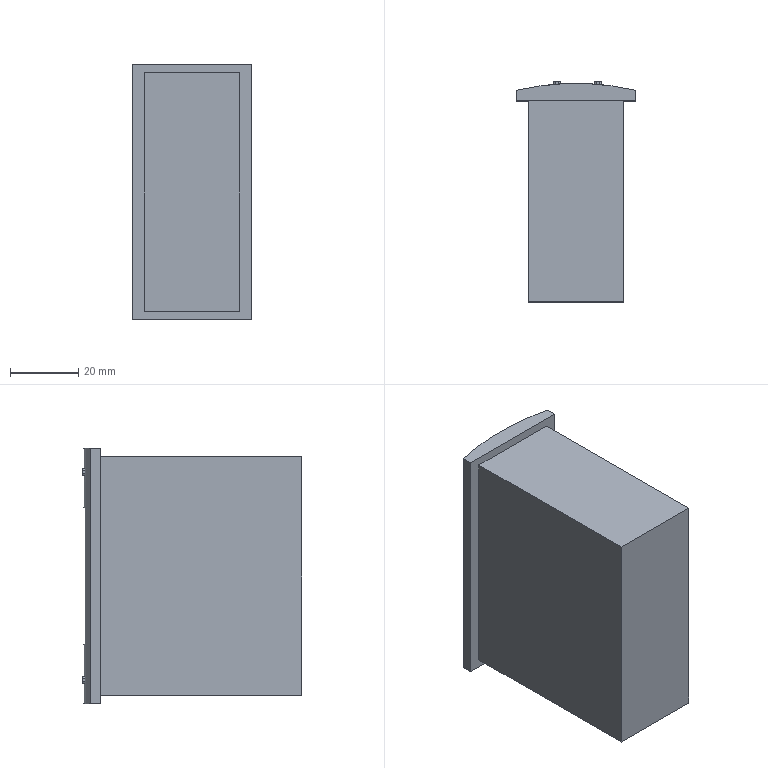Part | SolidWorks | features Fillet 4, ICE 3, Extrusion 1 | 5 solids | 56 faces | box 35 x 64.5 x 75 mm | volume 126879 mm3 | plane 39 | cylinder 17 | commonest cylinder face diameters 1 x16 152 x1
STEP:
#1=CARTESIAN_POINT('',(11.,5.5,68.5));
#2=VERTEX_POINT('',#1);
#3=CARTESIAN_POINT('',(11.,5.5,67.5));
#4=VERTEX_POINT('',#3);
#5=CARTESIAN_POINT('',(11.,5.5,69.));
#6=DIRECTION('',(0.,0.,-1.));
#7=VECTOR('',#6,1000.);
#8=LINE('',#5,#7);
#9=EDGE_CURVE('',#2,#4,#8,.T.);
#10=ORIENTED_EDGE('',*,*,#9,.T.);
#11=CARTESIAN_POINT('',(11.,3.,67.5));
#12=VERTEX_POINT('',#11);
#13=CARTESIAN_POINT('',(11.,5.5,67.5));
#14=DIRECTION('',(0.,-1.,0.));
#15=VECTOR('',#14,1000.);
#16=LINE('',#13,#15);
#17=EDGE_CURVE('',#4,#12,#16,.T.);
#18=ORIENTED_EDGE('',*,*,#17,.T.);
#19=CARTESIAN_POINT('',(11.,3.,68.5));
#20=VERTEX_POINT('',#19);
#21=CARTESIAN_POINT('',(11.,3.,69.));
#22=DIRECTION('',(0.,0.,-1.));
#23=VECTOR('',#22,1000.);
#24=LINE('',#21,#23);
#25=EDGE_CURVE('',#20,#12,#24,.T.);
#26=ORIENTED_EDGE('',*,*,#25,.F.);
#27=CARTESIAN_POINT('',(11.,5.5,68.5));
#28=DIRECTION('',(0.,1.,0.));
#29=VECTOR('',#28,1000.);
#30=LINE('',#27,#29);
#31=EDGE_CURVE('',#20,#2,#30,.T.);
#32=ORIENTED_EDGE('',*,*,#31,.T.);
#33=EDGE_LOOP('',(#10,#18,#26,#32));
#34=FACE_OUTER_BOUND('',#33,.T.);
#35=CARTESIAN_POINT('',(11.,5.5,69.));
#36=DIRECTION('',(-1.,0.,0.));
#37=DIRECTION('',(0.,0.,1.));
#38=AXIS2_PLACEMENT_3D('',#35,#36,#37);
#39=PLANE('',#38);
#40=ADVANCED_FACE('',(#34),#39,.T.);
#41=CARTESIAN_POINT('',(12.5,3.,69.));
#42=VERTEX_POINT('',#41);
#43=CARTESIAN_POINT('',(11.5,3.,69.));
#44=VERTEX_POINT('',#43);
#45=CARTESIAN_POINT('',(11.,3.,69.));
#46=DIRECTION('',(-1.,0.,0.));
#47=VECTOR('',#46,1000.);
#48=LINE('',#45,#47);
#49=EDGE_CURVE('',#42,#44,#48,.T.);
#50=ORIENTED_EDGE('',*,*,#49,.F.);
#51=CARTESIAN_POINT('',(12.5,5.5,69.));
#52=VERTEX_POINT('',#51);
#53=CARTESIAN_POINT('',(12.5,5.5,69.));
#54=DIRECTION('',(0.,1.,0.));
#55=VECTOR('',#54,1000.);
#56=LINE('',#53,#55);
#57=EDGE_CURVE('',#42,#52,#56,.T.);
#58=ORIENTED_EDGE('',*,*,#57,.T.);
#59=CARTESIAN_POINT('',(11.5,5.5,69.));
#60=VERTEX_POINT('',#59);
#61=CARTESIAN_POINT('',(11.,5.5,69.));
#62=DIRECTION('',(-1.,0.,0.));
#63=VECTOR('',#62,1000.);
#64=LINE('',#61,#63);
#65=EDGE_CURVE('',#52,#60,#64,.T.);
#66=ORIENTED_EDGE('',*,*,#65,.T.);
#67=CARTESIAN_POINT('',(11.5,5.5,69.));
#68=DIRECTION('',(0.,-1.,0.));
#69=VECTOR('',#68,1000.);
#70=LINE('',#67,#69);
#71=EDGE_CURVE('',#60,#44,#70,.T.);
#72=ORIENTED_EDGE('',*,*,#71,.T.);
#73=EDGE_LOOP('',(#50,#58,#66,#72));
#74=FACE_OUTER_BOUND('',#73,.T.);
#75=CARTESIAN_POINT('',(11.,5.5,69.));
#76=DIRECTION('',(0.,0.,1.));
#77=DIRECTION('',(1.,0.,0.));
#78=AXIS2_PLACEMENT_3D('',#75,#76,#77);
#79=PLANE('',#78);
#80=ADVANCED_FACE('',(#74),#79,.T.);
#81=CARTESIAN_POINT('',(13.,5.5,67.5));
#82=VERTEX_POINT('',#81);
#83=CARTESIAN_POINT('',(13.,5.5,68.5));
#84=VERTEX_POINT('',#83);
#85=CARTESIAN_POINT('',(13.,5.5,69.));
#86=DIRECTION('',(0.,0.,1.));
#87=VECTOR('',#86,1000.);
#88=LINE('',#85,#87);
#89=EDGE_CURVE('',#82,#84,#88,.T.);
#90=ORIENTED_EDGE('',*,*,#89,.T.);
#91=CARTESIAN_POINT('',(13.,3.,68.5));
#92=VERTEX_POINT('',#91);
#93=CARTESIAN_POINT('',(13.,5.5,68.5));
#94=DIRECTION('',(0.,-1.,0.));
#95=VECTOR('',#94,1000.);
#96=LINE('',#93,#95);
#97=EDGE_CURVE('',#84,#92,#96,.T.);
#98=ORIENTED_EDGE('',*,*,#97,.T.);
#99=CARTESIAN_POINT('',(13.,3.,67.5));
#100=VERTEX_POINT('',#99);
#101=CARTESIAN_POINT('',(13.,3.,69.));
#102=DIRECTION('',(0.,0.,1.));
#103=VECTOR('',#102,1000.);
#104=LINE('',#101,#103);
#105=EDGE_CURVE('',#100,#92,#104,.T.);
#106=ORIENTED_EDGE('',*,*,#105,.F.);
#107=CARTESIAN_POINT('',(13.,5.5,67.5));
#108=DIRECTION('',(0.,1.,0.));
#109=VECTOR('',#108,1000.);
#110=LINE('',#107,#109);
#111=EDGE_CURVE('',#100,#82,#110,.T.);
#112=ORIENTED_EDGE('',*,*,#111,.T.);
#113=EDGE_LOOP('',(#90,#98,#106,#112));
#114=FACE_OUTER_BOUND('',#113,.T.);
#115=CARTESIAN_POINT('',(13.,5.5,69.));
#116=DIRECTION('',(1.,0.,0.));
#117=DIRECTION('',(0.,0.,-1.));
#118=AXIS2_PLACEMENT_3D('',#115,#116,#117);
#119=PLANE('',#118);
#120=ADVANCED_FACE('',(#114),#119,.T.);
#121=CARTESIAN_POINT('',(11.5,5.5,67.));
#122=VERTEX_POINT('',#121);
#123=CARTESIAN_POINT('',(12.5,5.5,67.));
#124=VERTEX_POINT('',#123);
#125=CARTESIAN_POINT('',(11.,5.5,67.));
#126=DIRECTION('',(1.,0.,0.));
#127=VECTOR('',#126,1000.);
#128=LINE('',#125,#127);
#129=EDGE_CURVE('',#122,#124,#128,.T.);
#130=ORIENTED_EDGE('',*,*,#129,.T.);
#131=CARTESIAN_POINT('',(12.5,3.,67.));
#132=VERTEX_POINT('',#131);
#133=CARTESIAN_POINT('',(12.5,5.5,67.));
#134=DIRECTION('',(0.,-1.,0.));
#135=VECTOR('',#134,1000.);
#136=LINE('',#133,#135);
#137=EDGE_CURVE('',#124,#132,#136,.T.);
#138=ORIENTED_EDGE('',*,*,#137,.T.);
#139=CARTESIAN_POINT('',(11.5,3.,67.));
#140=VERTEX_POINT('',#139);
#141=CARTESIAN_POINT('',(11.,3.,67.));
#142=DIRECTION('',(1.,0.,0.));
#143=VECTOR('',#142,1000.);
#144=LINE('',#141,#143);
#145=EDGE_CURVE('',#140,#132,#144,.T.);
#146=ORIENTED_EDGE('',*,*,#145,.F.);
#147=CARTESIAN_POINT('',(11.5,5.5,67.));
#148=DIRECTION('',(0.,1.,0.));
#149=VECTOR('',#148,1000.);
#150=LINE('',#147,#149);
#151=EDGE_CURVE('',#140,#122,#150,.T.);
#152=ORIENTED_EDGE('',*,*,#151,.T.);
#153=EDGE_LOOP('',(#130,#138,#146,#152));
#154=FACE_OUTER_BOUND('',#153,.T.);
#155=CARTESIAN_POINT('',(11.,5.5,67.));
#156=DIRECTION('',(0.,0.,-1.));
#157=DIRECTION('',(-1.,0.,0.));
#158=AXIS2_PLACEMENT_3D('',#155,#156,#157);
#159=PLANE('',#158);
#160=ADVANCED_FACE('',(#154),#159,.T.);
#161=ORIENTED_EDGE('',*,*,#65,.F.);
#162=CARTESIAN_POINT('',(12.5,5.5,68.5));
#163=DIRECTION('',(0.,1.,0.));
#164=DIRECTION('',(0.,0.,-1.));
#165=AXIS2_PLACEMENT_3D('',#162,#163,#164);
#166=CIRCLE('',#165,0.5);
#167=EDGE_CURVE('',#52,#84,#166,.T.);
#168=ORIENTED_EDGE('',*,*,#167,.T.);
#169=ORIENTED_EDGE('',*,*,#89,.F.);
#170=CARTESIAN_POINT('',(12.5,5.5,67.5));
#171=DIRECTION('',(0.,1.,0.));
#172=DIRECTION('',(0.,0.,-1.));
#173=AXIS2_PLACEMENT_3D('',#170,#171,#172);
#174=CIRCLE('',#173,0.5);
#175=EDGE_CURVE('',#82,#124,#174,.T.);
#176=ORIENTED_EDGE('',*,*,#175,.T.);
#177=ORIENTED_EDGE('',*,*,#129,.F.);
#178=CARTESIAN_POINT('',(11.5,5.5,67.5));
#179=DIRECTION('',(0.,1.,0.));
#180=DIRECTION('',(0.,0.,-1.));
#181=AXIS2_PLACEMENT_3D('',#178,#179,#180);
#182=CIRCLE('',#181,0.5);
#183=EDGE_CURVE('',#122,#4,#182,.T.);
#184=ORIENTED_EDGE('',*,*,#183,.T.);
#185=ORIENTED_EDGE('',*,*,#9,.F.);
#186=CARTESIAN_POINT('',(11.5,5.5,68.5));
#187=DIRECTION('',(0.,1.,0.));
#188=DIRECTION('',(0.,0.,-1.));
#189=AXIS2_PLACEMENT_3D('',#186,#187,#188);
#190=CIRCLE('',#189,0.5);
#191=EDGE_CURVE('',#2,#60,#190,.T.);
#192=ORIENTED_EDGE('',*,*,#191,.T.);
#193=EDGE_LOOP('',(#161,#168,#169,#176,#177,#184,#185,#192));
#194=FACE_OUTER_BOUND('',#193,.T.);
#195=CARTESIAN_POINT('',(0.,5.5,0.));
#196=DIRECTION('',(0.,-1.,0.));
#197=DIRECTION('',(0.,0.,-1.));
#198=AXIS2_PLACEMENT_3D('',#195,#196,#197);
#199=PLANE('',#198);
#200=ADVANCED_FACE('',(#194),#199,.F.);
#201=ORIENTED_EDGE('',*,*,#105,.T.);
#202=CARTESIAN_POINT('',(12.5,3.,68.5));
#203=DIRECTION('',(0.,-1.,0.));
#204=DIRECTION('',(0.,0.,-1.));
#205=AXIS2_PLACEMENT_3D('',#202,#203,#204);
#206=CIRCLE('',#205,0.5);
#207=EDGE_CURVE('',#92,#42,#206,.T.);
#208=ORIENTED_EDGE('',*,*,#207,.T.);
#209=ORIENTED_EDGE('',*,*,#49,.T.);
#210=CARTESIAN_POINT('',(11.5,3.,68.5));
#211=DIRECTION('',(0.,-1.,0.));
#212=DIRECTION('',(0.,0.,-1.));
#213=AXIS2_PLACEMENT_3D('',#210,#211,#212);
#214=CIRCLE('',#213,0.5);
#215=EDGE_CURVE('',#44,#20,#214,.T.);
#216=ORIENTED_EDGE('',*,*,#215,.T.);
#217=ORIENTED_EDGE('',*,*,#25,.T.);
#218=CARTESIAN_POINT('',(11.5,3.,67.5));
#219=DIRECTION('',(0.,-1.,0.));
#220=DIRECTION('',(0.,0.,-1.));
#221=AXIS2_PLACEMENT_3D('',#218,#219,#220);
#222=CIRCLE('',#221,0.5);
#223=EDGE_CURVE('',#12,#140,#222,.T.);
#224=ORIENTED_EDGE('',*,*,#223,.T.);
#225=ORIENTED_EDGE('',*,*,#145,.T.);
#226=CARTESIAN_POINT('',(12.5,3.,67.5));
#227=DIRECTION('',(0.,-1.,0.));
#228=DIRECTION('',(0.,0.,-1.));
#229=AXIS2_PLACEMENT_3D('',#226,#227,#228);
#230=CIRCLE('',#229,0.5);
#231=EDGE_CURVE('',#132,#100,#230,.T.);
#232=ORIENTED_EDGE('',*,*,#231,.T.);
#233=EDGE_LOOP('',(#201,#208,#209,#216,#217,#224,#225,#232));
#234=FACE_OUTER_BOUND('',#233,.T.);
#235=CARTESIAN_POINT('',(0.,3.,0.));
#236=DIRECTION('',(0.,-1.,0.));
#237=DIRECTION('',(0.,0.,-1.));
#238=AXIS2_PLACEMENT_3D('',#235,#236,#237);
#239=PLANE('',#238);
#240=ADVANCED_FACE('',(#234),#239,.T.);
#241=ORIENTED_EDGE('',*,*,#167,.F.);
#242=ORIENTED_EDGE('',*,*,#57,.F.);
#243=ORIENTED_EDGE('',*,*,#207,.F.);
#244=ORIENTED_EDGE('',*,*,#97,.F.);
#245=EDGE_LOOP('',(#241,#242,#243,#244));
#246=FACE_OUTER_BOUND('',#245,.T.);
#247=CARTESIAN_POINT('',(12.5,5.5,68.5));
#248=DIRECTION('',(0.,-1.,0.));
#249=DIRECTION('',(0.,0.,-1.));
#250=AXIS2_PLACEMENT_3D('',#247,#248,#249);
#251=CYLINDRICAL_SURFACE('',#250,0.5);
#252=ADVANCED_FACE('',(#246),#251,.T.);
#253=ORIENTED_EDGE('',*,*,#175,.F.);
#254=ORIENTED_EDGE('',*,*,#111,.F.);
#255=ORIENTED_EDGE('',*,*,#231,.F.);
#256=ORIENTED_EDGE('',*,*,#137,.F.);
#257=EDGE_LOOP('',(#253,#254,#255,#256));
#258=FACE_OUTER_BOUND('',#257,.T.);
#259=CARTESIAN_POINT('',(12.5,5.5,67.5));
#260=DIRECTION('',(0.,-1.,0.));
#261=DIRECTION('',(0.,0.,-1.));
#262=AXIS2_PLACEMENT_3D('',#259,#260,#261);
#263=CYLINDRICAL_SURFACE('',#262,0.5);
#264=ADVANCED_FACE('',(#258),#263,.T.);
#265=ORIENTED_EDGE('',*,*,#183,.F.);
#266=ORIENTED_EDGE('',*,*,#151,.F.);
#267=ORIENTED_EDGE('',*,*,#223,.F.);
#268=ORIENTED_EDGE('',*,*,#17,.F.);
#269=EDGE_LOOP('',(#265,#266,#267,#268));
#270=FACE_OUTER_BOUND('',#269,.T.);
#271=CARTESIAN_POINT('',(11.5,5.5,67.5));
#272=DIRECTION('',(0.,-1.,0.));
#273=DIRECTION('',(0.,0.,-1.));
#274=AXIS2_PLACEMENT_3D('',#271,#272,#273);
#275=CYLINDRICAL_SURFACE('',#274,0.5);
#276=ADVANCED_FACE('',(#270),#275,.T.);
#277=ORIENTED_EDGE('',*,*,#191,.F.);
#278=ORIENTED_EDGE('',*,*,#31,.F.);
#279=ORIENTED_EDGE('',*,*,#215,.F.);
#280=ORIENTED_EDGE('',*,*,#71,.F.);
#281=EDGE_LOOP('',(#277,#278,#279,#280));
#282=FACE_OUTER_BOUND('',#281,.T.);
#283=CARTESIAN_POINT('',(11.5,5.5,68.5));
#284=DIRECTION('',(0.,-1.,0.));
#285=DIRECTION('',(0.,0.,-1.));
#286=AXIS2_PLACEMENT_3D('',#283,#284,#285);
#287=CYLINDRICAL_SURFACE('',#286,0.5);
#288=ADVANCED_FACE('',(#282),#287,.T.);
#289=CLOSED_SHELL('',(#40,#80,#120,#160,#200,#240,#252,#264,#276,#288));
#290=MANIFOLD_SOLID_BREP('',#289);
#291=CARTESIAN_POINT('',(23.,5.5,68.5));
#292=VERTEX_POINT('',#291);
#293=CARTESIAN_POINT('',(23.,5.5,67.5));
#294=VERTEX_POINT('',#293);
#295=CARTESIAN_POINT('',(23.,5.5,69.));
#296=DIRECTION('',(0.,0.,-1.));
#297=VECTOR('',#296,1000.);
#298=LINE('',#295,#297);
#299=EDGE_CURVE('',#292,#294,#298,.T.);
#300=ORIENTED_EDGE('',*,*,#299,.T.);
#301=CARTESIAN_POINT('',(23.,3.,67.5));
#302=VERTEX_POINT('',#301);
#303=CARTESIAN_POINT('',(23.,5.5,67.5));
#304=DIRECTION('',(0.,-1.,0.));
#305=VECTOR('',#304,1000.);
#306=LINE('',#303,#305);
#307=EDGE_CURVE('',#294,#302,#306,.T.);
#308=ORIENTED_EDGE('',*,*,#307,.T.);
#309=CARTESIAN_POINT('',(23.,3.,68.5));
#310=VERTEX_POINT('',#309);
#311=CARTESIAN_POINT('',(23.,3.,69.));
#312=DIRECTION('',(0.,0.,-1.));
#313=VECTOR('',#312,1000.);
#314=LINE('',#311,#313);
#315=EDGE_CURVE('',#310,#302,#314,.T.);
#316=ORIENTED_EDGE('',*,*,#315,.F.);
#317=CARTESIAN_POINT('',(23.,5.5,68.5));
#318=DIRECTION('',(0.,1.,0.));
#319=VECTOR('',#318,1000.);
#320=LINE('',#317,#319);
#321=EDGE_CURVE('',#310,#292,#320,.T.);
#322=ORIENTED_EDGE('',*,*,#321,.T.);
#323=EDGE_LOOP('',(#300,#308,#316,#322));
#324=FACE_OUTER_BOUND('',#323,.T.);
#325=CARTESIAN_POINT('',(23.,5.5,69.));
#326=DIRECTION('',(-1.,0.,0.));
#327=DIRECTION('',(0.,0.,1.));
#328=AXIS2_PLACEMENT_3D('',#325,#326,#327);
#329=PLANE('',#328);
#330=ADVANCED_FACE('',(#324),#329,.T.);
#331=CARTESIAN_POINT('',(24.5,3.,69.));
#332=VERTEX_POINT('',#331);
#333=CARTESIAN_POINT('',(23.5,3.,69.));
#334=VERTEX_POINT('',#333);
#335=CARTESIAN_POINT('',(23.,3.,69.));
#336=DIRECTION('',(-1.,0.,0.));
#337=VECTOR('',#336,1000.);
#338=LINE('',#335,#337);
#339=EDGE_CURVE('',#332,#334,#338,.T.);
#340=ORIENTED_EDGE('',*,*,#339,.F.);
#341=CARTESIAN_POINT('',(24.5,5.5,69.));
#342=VERTEX_POINT('',#341);
#343=CARTESIAN_POINT('',(24.5,5.5,69.));
#344=DIRECTION('',(0.,1.,0.));
#345=VECTOR('',#344,1000.);
#346=LINE('',#343,#345);
#347=EDGE_CURVE('',#332,#342,#346,.T.);
#348=ORIENTED_EDGE('',*,*,#347,.T.);
#349=CARTESIAN_POINT('',(23.5,5.5,69.));
#350=VERTEX_POINT('',#349);
#351=CARTESIAN_POINT('',(23.,5.5,69.));
#352=DIRECTION('',(-1.,0.,0.));
#353=VECTOR('',#352,1000.);
#354=LINE('',#351,#353);
#355=EDGE_CURVE('',#342,#350,#354,.T.);
#356=ORIENTED_EDGE('',*,*,#355,.T.);
#357=CARTESIAN_POINT('',(23.5,5.5,69.));
#358=DIRECTION('',(0.,-1.,0.));
#359=VECTOR('',#358,1000.);
#360=LINE('',#357,#359);
#361=EDGE_CURVE('',#350,#334,#360,.T.);
#362=ORIENTED_EDGE('',*,*,#361,.T.);
#363=EDGE_LOOP('',(#340,#348,#356,#362));
#364=FACE_OUTER_BOUND('',#363,.T.);
#365=CARTESIAN_POINT('',(23.,5.5,69.));
#366=DIRECTION('',(0.,0.,1.));
#367=DIRECTION('',(1.,0.,0.));
#368=AXIS2_PLACEMENT_3D('',#365,#366,#367);
#369=PLANE('',#368);
#370=ADVANCED_FACE('',(#364),#369,.T.);
#371=CARTESIAN_POINT('',(25.,5.5,67.5));
#372=VERTEX_POINT('',#371);
#373=CARTESIAN_POINT('',(25.,5.5,68.5));
#374=VERTEX_POINT('',#373);
#375=CARTESIAN_POINT('',(25.,5.5,69.));
#376=DIRECTION('',(0.,0.,1.));
#377=VECTOR('',#376,1000.);
#378=LINE('',#375,#377);
#379=EDGE_CURVE('',#372,#374,#378,.T.);
#380=ORIENTED_EDGE('',*,*,#379,.T.);
#381=CARTESIAN_POINT('',(25.,3.,68.5));
#382=VERTEX_POINT('',#381);
#383=CARTESIAN_POINT('',(25.,5.5,68.5));
#384=DIRECTION('',(0.,-1.,0.));
#385=VECTOR('',#384,1000.);
#386=LINE('',#383,#385);
#387=EDGE_CURVE('',#374,#382,#386,.T.);
#388=ORIENTED_EDGE('',*,*,#387,.T.);
#389=CARTESIAN_POINT('',(25.,3.,67.5));
#390=VERTEX_POINT('',#389);
#391=CARTESIAN_POINT('',(25.,3.,69.));
#392=DIRECTION('',(0.,0.,1.));
#393=VECTOR('',#392,1000.);
#394=LINE('',#391,#393);
#395=EDGE_CURVE('',#390,#382,#394,.T.);
#396=ORIENTED_EDGE('',*,*,#395,.F.);
#397=CARTESIAN_POINT('',(25.,5.5,67.5));
#398=DIRECTION('',(0.,1.,0.));
#399=VECTOR('',#398,1000.);
#400=LINE('',#397,#399);
#401=EDGE_CURVE('',#390,#372,#400,.T.);
#402=ORIENTED_EDGE('',*,*,#401,.T.);
#403=EDGE_LOOP('',(#380,#388,#396,#402));
#404=FACE_OUTER_BOUND('',#403,.T.);
#405=CARTESIAN_POINT('',(25.,5.5,69.));
#406=DIRECTION('',(1.,0.,0.));
#407=DIRECTION('',(0.,0.,-1.));
#408=AXIS2_PLACEMENT_3D('',#405,#406,#407);
#409=PLANE('',#408);
#410=ADVANCED_FACE('',(#404),#409,.T.);
#411=CARTESIAN_POINT('',(23.5,5.5,67.));
#412=VERTEX_POINT('',#411);
#413=CARTESIAN_POINT('',(24.5,5.5,67.));
#414=VERTEX_POINT('',#413);
#415=CARTESIAN_POINT('',(23.,5.5,67.));
#416=DIRECTION('',(1.,0.,0.));
#417=VECTOR('',#416,1000.);
#418=LINE('',#415,#417);
#419=EDGE_CURVE('',#412,#414,#418,.T.);
#420=ORIENTED_EDGE('',*,*,#419,.T.);
#421=CARTESIAN_POINT('',(24.5,3.,67.));
#422=VERTEX_POINT('',#421);
#423=CARTESIAN_POINT('',(24.5,5.5,67.));
#424=DIRECTION('',(0.,-1.,0.));
#425=VECTOR('',#424,1000.);
#426=LINE('',#423,#425);
#427=EDGE_CURVE('',#414,#422,#426,.T.);
#428=ORIENTED_EDGE('',*,*,#427,.T.);
#429=CARTESIAN_POINT('',(23.5,3.,67.));
#430=VERTEX_POINT('',#429);
#431=CARTESIAN_POINT('',(23.,3.,67.));
#432=DIRECTION('',(1.,0.,0.));
#433=VECTOR('',#432,1000.);
#434=LINE('',#431,#433);
#435=EDGE_CURVE('',#430,#422,#434,.T.);
#436=ORIENTED_EDGE('',*,*,#435,.F.);
#437=CARTESIAN_POINT('',(23.5,5.5,67.));
#438=DIRECTION('',(0.,1.,0.));
#439=VECTOR('',#438,1000.);
#440=LINE('',#437,#439);
#441=EDGE_CURVE('',#430,#412,#440,.T.);
#442=ORIENTED_EDGE('',*,*,#441,.T.);
#443=EDGE_LOOP('',(#420,#428,#436,#442));
#444=FACE_OUTER_BOUND('',#443,.T.);
#445=CARTESIAN_POINT('',(23.,5.5,67.));
#446=DIRECTION('',(0.,0.,-1.));
#447=DIRECTION('',(-1.,0.,0.));
#448=AXIS2_PLACEMENT_3D('',#445,#446,#447);
#449=PLANE('',#448);
#450=ADVANCED_FACE('',(#444),#449,.T.);
#451=ORIENTED_EDGE('',*,*,#355,.F.);
#452=CARTESIAN_POINT('',(24.5,5.5,68.5));
#453=DIRECTION('',(0.,1.,0.));
#454=DIRECTION('',(0.,0.,-1.));
#455=AXIS2_PLACEMENT_3D('',#452,#453,#454);
#456=CIRCLE('',#455,0.5);
#457=EDGE_CURVE('',#342,#374,#456,.T.);
#458=ORIENTED_EDGE('',*,*,#457,.T.);
#459=ORIENTED_EDGE('',*,*,#379,.F.);
#460=CARTESIAN_POINT('',(24.5,5.5,67.5));
#461=DIRECTION('',(0.,1.,0.));
#462=DIRECTION('',(0.,0.,-1.));
#463=AXIS2_PLACEMENT_3D('',#460,#461,#462);
#464=CIRCLE('',#463,0.5);
#465=EDGE_CURVE('',#372,#414,#464,.T.);
#466=ORIENTED_EDGE('',*,*,#465,.T.);
#467=ORIENTED_EDGE('',*,*,#419,.F.);
#468=CARTESIAN_POINT('',(23.5,5.5,67.5));
#469=DIRECTION('',(0.,1.,0.));
#470=DIRECTION('',(0.,0.,-1.));
#471=AXIS2_PLACEMENT_3D('',#468,#469,#470);
#472=CIRCLE('',#471,0.5);
#473=EDGE_CURVE('',#412,#294,#472,.T.);
#474=ORIENTED_EDGE('',*,*,#473,.T.);
#475=ORIENTED_EDGE('',*,*,#299,.F.);
#476=CARTESIAN_POINT('',(23.5,5.5,68.5));
#477=DIRECTION('',(0.,1.,0.));
#478=DIRECTION('',(0.,0.,-1.));
#479=AXIS2_PLACEMENT_3D('',#476,#477,#478);
#480=CIRCLE('',#479,0.5);
#481=EDGE_CURVE('',#292,#350,#480,.T.);
#482=ORIENTED_EDGE('',*,*,#481,.T.);
#483=EDGE_LOOP('',(#451,#458,#459,#466,#467,#474,#475,#482));
#484=FACE_OUTER_BOUND('',#483,.T.);
#485=CARTESIAN_POINT('',(0.,5.5,0.));
#486=DIRECTION('',(0.,-1.,0.));
#487=DIRECTION('',(0.,0.,-1.));
#488=AXIS2_PLACEMENT_3D('',#485,#486,#487);
#489=PLANE('',#488);
#490=ADVANCED_FACE('',(#484),#489,.F.);
#491=ORIENTED_EDGE('',*,*,#395,.T.);
#492=CARTESIAN_POINT('',(24.5,3.,68.5));
#493=DIRECTION('',(0.,-1.,0.));
#494=DIRECTION('',(0.,0.,-1.));
#495=AXIS2_PLACEMENT_3D('',#492,#493,#494);
#496=CIRCLE('',#495,0.5);
#497=EDGE_CURVE('',#382,#332,#496,.T.);
#498=ORIENTED_EDGE('',*,*,#497,.T.);
#499=ORIENTED_EDGE('',*,*,#339,.T.);
#500=CARTESIAN_POINT('',(23.5,3.,68.5));
#501=DIRECTION('',(0.,-1.,0.));
#502=DIRECTION('',(0.,0.,-1.));
#503=AXIS2_PLACEMENT_3D('',#500,#501,#502);
#504=CIRCLE('',#503,0.5);
#505=EDGE_CURVE('',#334,#310,#504,.T.);
#506=ORIENTED_EDGE('',*,*,#505,.T.);
#507=ORIENTED_EDGE('',*,*,#315,.T.);
#508=CARTESIAN_POINT('',(23.5,3.,67.5));
#509=DIRECTION('',(0.,-1.,0.));
#510=DIRECTION('',(0.,0.,-1.));
#511=AXIS2_PLACEMENT_3D('',#508,#509,#510);
#512=CIRCLE('',#511,0.5);
#513=EDGE_CURVE('',#302,#430,#512,.T.);
#514=ORIENTED_EDGE('',*,*,#513,.T.);
#515=ORIENTED_EDGE('',*,*,#435,.T.);
#516=CARTESIAN_POINT('',(24.5,3.,67.5));
#517=DIRECTION('',(0.,-1.,0.));
#518=DIRECTION('',(0.,0.,-1.));
#519=AXIS2_PLACEMENT_3D('',#516,#517,#518);
#520=CIRCLE('',#519,0.5);
#521=EDGE_CURVE('',#422,#390,#520,.T.);
#522=ORIENTED_EDGE('',*,*,#521,.T.);
#523=EDGE_LOOP('',(#491,#498,#499,#506,#507,#514,#515,#522));
#524=FACE_OUTER_BOUND('',#523,.T.);
#525=CARTESIAN_POINT('',(0.,3.,0.));
#526=DIRECTION('',(0.,-1.,0.));
#527=DIRECTION('',(0.,0.,-1.));
#528=AXIS2_PLACEMENT_3D('',#525,#526,#527);
#529=PLANE('',#528);
#530=ADVANCED_FACE('',(#524),#529,.T.);
#531=ORIENTED_EDGE('',*,*,#457,.F.);
#532=ORIENTED_EDGE('',*,*,#347,.F.);
#533=ORIENTED_EDGE('',*,*,#497,.F.);
#534=ORIENTED_EDGE('',*,*,#387,.F.);
#535=EDGE_LOOP('',(#531,#532,#533,#534));
#536=FACE_OUTER_BOUND('',#535,.T.);
#537=CARTESIAN_POINT('',(24.5,5.5,68.5));
#538=DIRECTION('',(0.,-1.,0.));
#539=DIRECTION('',(0.,0.,-1.));
#540=AXIS2_PLACEMENT_3D('',#537,#538,#539);
#541=CYLINDRICAL_SURFACE('',#540,0.5);
#542=ADVANCED_FACE('',(#536),#541,.T.);
#543=ORIENTED_EDGE('',*,*,#465,.F.);
#544=ORIENTED_EDGE('',*,*,#401,.F.);
#545=ORIENTED_EDGE('',*,*,#521,.F.);
#546=ORIENTED_EDGE('',*,*,#427,.F.);
#547=EDGE_LOOP('',(#543,#544,#545,#546));
#548=FACE_OUTER_BOUND('',#547,.T.);
#549=CARTESIAN_POINT('',(24.5,5.5,67.5));
#550=DIRECTION('',(0.,-1.,0.));
#551=DIRECTION('',(0.,0.,-1.));
#552=AXIS2_PLACEMENT_3D('',#549,#550,#551);
#553=CYLINDRICAL_SURFACE('',#552,0.5);
#554=ADVANCED_FACE('',(#548),#553,.T.);
#555=ORIENTED_EDGE('',*,*,#473,.F.);
#556=ORIENTED_EDGE('',*,*,#441,.F.);
#557=ORIENTED_EDGE('',*,*,#513,.F.);
#558=ORIENTED_EDGE('',*,*,#307,.F.);
#559=EDGE_LOOP('',(#555,#556,#557,#558));
#560=FACE_OUTER_BOUND('',#559,.T.);
#561=CARTESIAN_POINT('',(23.5,5.5,67.5));
#562=DIRECTION('',(0.,-1.,0.));
#563=DIRECTION('',(0.,0.,-1.));
#564=AXIS2_PLACEMENT_3D('',#561,#562,#563);
#565=CYLINDRICAL_SURFACE('',#564,0.5);
#566=ADVANCED_FACE('',(#560),#565,.T.);
#567=ORIENTED_EDGE('',*,*,#481,.F.);
#568=ORIENTED_EDGE('',*,*,#321,.F.);
#569=ORIENTED_EDGE('',*,*,#505,.F.);
#570=ORIENTED_EDGE('',*,*,#361,.F.);
#571=EDGE_LOOP('',(#567,#568,#569,#570));
#572=FACE_OUTER_BOUND('',#571,.T.);
#573=CARTESIAN_POINT('',(23.5,5.5,68.5));
#574=DIRECTION('',(0.,-1.,0.));
#575=DIRECTION('',(0.,0.,-1.));
#576=AXIS2_PLACEMENT_3D('',#573,#574,#575);
#577=CYLINDRICAL_SURFACE('',#576,0.5);
#578=ADVANCED_FACE('',(#572),#577,.T.);
#579=CLOSED_SHELL('',(#330,#370,#410,#450,#490,#530,#542,#554,#566,#578));
#580=MANIFOLD_SOLID_BREP('',#579);
#581=CARTESIAN_POINT('',(11.,3.,7.5));
#582=VERTEX_POINT('',#581);
#583=CARTESIAN_POINT('',(11.,3.,6.5));
#584=VERTEX_POINT('',#583);
#585=CARTESIAN_POINT('',(11.,3.,8.));
#586=DIRECTION('',(0.,0.,-1.));
#587=VECTOR('',#586,1000.);
#588=LINE('',#585,#587);
#589=EDGE_CURVE('',#582,#584,#588,.T.);
#590=ORIENTED_EDGE('',*,*,#589,.F.);
#591=CARTESIAN_POINT('',(11.,5.5,7.5));
#592=VERTEX_POINT('',#591);
#593=CARTESIAN_POINT('',(11.,5.5,7.5));
#594=DIRECTION('',(0.,1.,0.));
#595=VECTOR('',#594,1000.);
#596=LINE('',#593,#595);
#597=EDGE_CURVE('',#582,#592,#596,.T.);
#598=ORIENTED_EDGE('',*,*,#597,.T.);
#599=CARTESIAN_POINT('',(11.,5.5,6.5));
#600=VERTEX_POINT('',#599);
#601=CARTESIAN_POINT('',(11.,5.5,8.));
#602=DIRECTION('',(0.,0.,-1.));
#603=VECTOR('',#602,1000.);
#604=LINE('',#601,#603);
#605=EDGE_CURVE('',#592,#600,#604,.T.);
#606=ORIENTED_EDGE('',*,*,#605,.T.);
#607=CARTESIAN_POINT('',(11.,5.5,6.5));
#608=DIRECTION('',(0.,-1.,0.));
#609=VECTOR('',#608,1000.);
#610=LINE('',#607,#609);
#611=EDGE_CURVE('',#600,#584,#610,.T.);
#612=ORIENTED_EDGE('',*,*,#611,.T.);
#613=EDGE_LOOP('',(#590,#598,#606,#612));
#614=FACE_OUTER_BOUND('',#613,.T.);
#615=CARTESIAN_POINT('',(11.,5.5,8.));
#616=DIRECTION('',(-1.,0.,0.));
#617=DIRECTION('',(0.,0.,1.));
#618=AXIS2_PLACEMENT_3D('',#615,#616,#617);
#619=PLANE('',#618);
#620=ADVANCED_FACE('',(#614),#619,.T.);
#621=CARTESIAN_POINT('',(12.5,5.5,8.));
#622=VERTEX_POINT('',#621);
#623=CARTESIAN_POINT('',(11.5,5.5,8.));
#624=VERTEX_POINT('',#623);
#625=CARTESIAN_POINT('',(11.,5.5,8.));
#626=DIRECTION('',(-1.,0.,0.));
#627=VECTOR('',#626,1000.);
#628=LINE('',#625,#627);
#629=EDGE_CURVE('',#622,#624,#628,.T.);
#630=ORIENTED_EDGE('',*,*,#629,.T.);
#631=CARTESIAN_POINT('',(11.5,3.,8.));
#632=VERTEX_POINT('',#631);
#633=CARTESIAN_POINT('',(11.5,5.5,8.));
#634=DIRECTION('',(0.,-1.,0.));
#635=VECTOR('',#634,1000.);
#636=LINE('',#633,#635);
#637=EDGE_CURVE('',#624,#632,#636,.T.);
#638=ORIENTED_EDGE('',*,*,#637,.T.);
#639=CARTESIAN_POINT('',(12.5,3.,8.));
#640=VERTEX_POINT('',#639);
#641=CARTESIAN_POINT('',(11.,3.,8.));
#642=DIRECTION('',(-1.,0.,0.));
#643=VECTOR('',#642,1000.);
#644=LINE('',#641,#643);
#645=EDGE_CURVE('',#640,#632,#644,.T.);
#646=ORIENTED_EDGE('',*,*,#645,.F.);
#647=CARTESIAN_POINT('',(12.5,5.5,8.));
#648=DIRECTION('',(0.,1.,0.));
#649=VECTOR('',#648,1000.);
#650=LINE('',#647,#649);
#651=EDGE_CURVE('',#640,#622,#650,.T.);
#652=ORIENTED_EDGE('',*,*,#651,.T.);
#653=EDGE_LOOP('',(#630,#638,#646,#652));
#654=FACE_OUTER_BOUND('',#653,.T.);
#655=CARTESIAN_POINT('',(11.,5.5,8.));
#656=DIRECTION('',(0.,0.,1.));
#657=DIRECTION('',(1.,0.,0.));
#658=AXIS2_PLACEMENT_3D('',#655,#656,#657);
#659=PLANE('',#658);
#660=ADVANCED_FACE('',(#654),#659,.T.);
#661=CARTESIAN_POINT('',(13.,5.5,6.5));
#662=VERTEX_POINT('',#661);
#663=CARTESIAN_POINT('',(13.,5.5,7.5));
#664=VERTEX_POINT('',#663);
#665=CARTESIAN_POINT('',(13.,5.5,8.));
#666=DIRECTION('',(0.,0.,1.));
#667=VECTOR('',#666,1000.);
#668=LINE('',#665,#667);
#669=EDGE_CURVE('',#662,#664,#668,.T.);
#670=ORIENTED_EDGE('',*,*,#669,.T.);
#671=CARTESIAN_POINT('',(13.,3.,7.5));
#672=VERTEX_POINT('',#671);
#673=CARTESIAN_POINT('',(13.,5.5,7.5));
#674=DIRECTION('',(0.,-1.,0.));
#675=VECTOR('',#674,1000.);
#676=LINE('',#673,#675);
#677=EDGE_CURVE('',#664,#672,#676,.T.);
#678=ORIENTED_EDGE('',*,*,#677,.T.);
#679=CARTESIAN_POINT('',(13.,3.,6.5));
#680=VERTEX_POINT('',#679);
#681=CARTESIAN_POINT('',(13.,3.,8.));
#682=DIRECTION('',(0.,0.,1.));
#683=VECTOR('',#682,1000.);
#684=LINE('',#681,#683);
#685=EDGE_CURVE('',#680,#672,#684,.T.);
#686=ORIENTED_EDGE('',*,*,#685,.F.);
#687=CARTESIAN_POINT('',(13.,5.5,6.5));
#688=DIRECTION('',(0.,1.,0.));
#689=VECTOR('',#688,1000.);
#690=LINE('',#687,#689);
#691=EDGE_CURVE('',#680,#662,#690,.T.);
#692=ORIENTED_EDGE('',*,*,#691,.T.);
#693=EDGE_LOOP('',(#670,#678,#686,#692));
#694=FACE_OUTER_BOUND('',#693,.T.);
#695=CARTESIAN_POINT('',(13.,5.5,8.));
#696=DIRECTION('',(1.,0.,0.));
#697=DIRECTION('',(0.,0.,-1.));
#698=AXIS2_PLACEMENT_3D('',#695,#696,#697);
#699=PLANE('',#698);
#700=ADVANCED_FACE('',(#694),#699,.T.);
#701=CARTESIAN_POINT('',(11.5,5.5,6.));
#702=VERTEX_POINT('',#701);
#703=CARTESIAN_POINT('',(12.5,5.5,6.));
#704=VERTEX_POINT('',#703);
#705=CARTESIAN_POINT('',(11.,5.5,6.));
#706=DIRECTION('',(1.,0.,0.));
#707=VECTOR('',#706,1000.);
#708=LINE('',#705,#707);
#709=EDGE_CURVE('',#702,#704,#708,.T.);
#710=ORIENTED_EDGE('',*,*,#709,.T.);
#711=CARTESIAN_POINT('',(12.5,3.,6.));
#712=VERTEX_POINT('',#711);
#713=CARTESIAN_POINT('',(12.5,5.5,6.));
#714=DIRECTION('',(0.,-1.,0.));
#715=VECTOR('',#714,1000.);
#716=LINE('',#713,#715);
#717=EDGE_CURVE('',#704,#712,#716,.T.);
#718=ORIENTED_EDGE('',*,*,#717,.T.);
#719=CARTESIAN_POINT('',(11.5,3.,6.));
#720=VERTEX_POINT('',#719);
#721=CARTESIAN_POINT('',(11.,3.,6.));
#722=DIRECTION('',(1.,0.,0.));
#723=VECTOR('',#722,1000.);
#724=LINE('',#721,#723);
#725=EDGE_CURVE('',#720,#712,#724,.T.);
#726=ORIENTED_EDGE('',*,*,#725,.F.);
#727=CARTESIAN_POINT('',(11.5,5.5,6.));
#728=DIRECTION('',(0.,1.,0.));
#729=VECTOR('',#728,1000.);
#730=LINE('',#727,#729);
#731=EDGE_CURVE('',#720,#702,#730,.T.);
#732=ORIENTED_EDGE('',*,*,#731,.T.);
#733=EDGE_LOOP('',(#710,#718,#726,#732));
#734=FACE_OUTER_BOUND('',#733,.T.);
#735=CARTESIAN_POINT('',(11.,5.5,6.));
#736=DIRECTION('',(0.,0.,-1.));
#737=DIRECTION('',(-1.,0.,0.));
#738=AXIS2_PLACEMENT_3D('',#735,#736,#737);
#739=PLANE('',#738);
#740=ADVANCED_FACE('',(#734),#739,.T.);
#741=ORIENTED_EDGE('',*,*,#605,.F.);
#742=CARTESIAN_POINT('',(11.5,5.5,7.5));
#743=DIRECTION('',(0.,1.,0.));
#744=DIRECTION('',(0.,0.,-1.));
#745=AXIS2_PLACEMENT_3D('',#742,#743,#744);
#746=CIRCLE('',#745,0.5);
#747=EDGE_CURVE('',#592,#624,#746,.T.);
#748=ORIENTED_EDGE('',*,*,#747,.T.);
#749=ORIENTED_EDGE('',*,*,#629,.F.);
#750=CARTESIAN_POINT('',(12.5,5.5,7.5));
#751=DIRECTION('',(0.,1.,0.));
#752=DIRECTION('',(0.,0.,-1.));
#753=AXIS2_PLACEMENT_3D('',#750,#751,#752);
#754=CIRCLE('',#753,0.5);
#755=EDGE_CURVE('',#622,#664,#754,.T.);
#756=ORIENTED_EDGE('',*,*,#755,.T.);
#757=ORIENTED_EDGE('',*,*,#669,.F.);
#758=CARTESIAN_POINT('',(12.5,5.5,6.5));
#759=DIRECTION('',(0.,1.,0.));
#760=DIRECTION('',(0.,0.,-1.));
#761=AXIS2_PLACEMENT_3D('',#758,#759,#760);
#762=CIRCLE('',#761,0.5);
#763=EDGE_CURVE('',#662,#704,#762,.T.);
#764=ORIENTED_EDGE('',*,*,#763,.T.);
#765=ORIENTED_EDGE('',*,*,#709,.F.);
#766=CARTESIAN_POINT('',(11.5,5.5,6.5));
#767=DIRECTION('',(0.,1.,0.));
#768=DIRECTION('',(0.,0.,-1.));
#769=AXIS2_PLACEMENT_3D('',#766,#767,#768);
#770=CIRCLE('',#769,0.5);
#771=EDGE_CURVE('',#702,#600,#770,.T.);
#772=ORIENTED_EDGE('',*,*,#771,.T.);
#773=EDGE_LOOP('',(#741,#748,#749,#756,#757,#764,#765,#772));
#774=FACE_OUTER_BOUND('',#773,.T.);
#775=CARTESIAN_POINT('',(0.,5.5,0.));
#776=DIRECTION('',(0.,-1.,0.));
#777=DIRECTION('',(0.,0.,-1.));
#778=AXIS2_PLACEMENT_3D('',#775,#776,#777);
#779=PLANE('',#778);
#780=ADVANCED_FACE('',(#774),#779,.F.);
#781=ORIENTED_EDGE('',*,*,#645,.T.);
#782=CARTESIAN_POINT('',(11.5,3.,7.5));
#783=DIRECTION('',(0.,-1.,0.));
#784=DIRECTION('',(0.,0.,-1.));
#785=AXIS2_PLACEMENT_3D('',#782,#783,#784);
#786=CIRCLE('',#785,0.5);
#787=EDGE_CURVE('',#632,#582,#786,.T.);
#788=ORIENTED_EDGE('',*,*,#787,.T.);
#789=ORIENTED_EDGE('',*,*,#589,.T.);
#790=CARTESIAN_POINT('',(11.5,3.,6.5));
#791=DIRECTION('',(0.,-1.,0.));
#792=DIRECTION('',(0.,0.,-1.));
#793=AXIS2_PLACEMENT_3D('',#790,#791,#792);
#794=CIRCLE('',#793,0.5);
#795=EDGE_CURVE('',#584,#720,#794,.T.);
#796=ORIENTED_EDGE('',*,*,#795,.T.);
#797=ORIENTED_EDGE('',*,*,#725,.T.);
#798=CARTESIAN_POINT('',(12.5,3.,6.5));
#799=DIRECTION('',(0.,-1.,0.));
#800=DIRECTION('',(0.,0.,-1.));
#801=AXIS2_PLACEMENT_3D('',#798,#799,#800);
#802=CIRCLE('',#801,0.5);
#803=EDGE_CURVE('',#712,#680,#802,.T.);
#804=ORIENTED_EDGE('',*,*,#803,.T.);
#805=ORIENTED_EDGE('',*,*,#685,.T.);
#806=CARTESIAN_POINT('',(12.5,3.,7.5));
#807=DIRECTION('',(0.,-1.,0.));
#808=DIRECTION('',(0.,0.,-1.));
#809=AXIS2_PLACEMENT_3D('',#806,#807,#808);
#810=CIRCLE('',#809,0.5);
#811=EDGE_CURVE('',#672,#640,#810,.T.);
#812=ORIENTED_EDGE('',*,*,#811,.T.);
#813=EDGE_LOOP('',(#781,#788,#789,#796,#797,#804,#805,#812));
#814=FACE_OUTER_BOUND('',#813,.T.);
#815=CARTESIAN_POINT('',(0.,3.,0.));
#816=DIRECTION('',(0.,-1.,0.));
#817=DIRECTION('',(0.,0.,-1.));
#818=AXIS2_PLACEMENT_3D('',#815,#816,#817);
#819=PLANE('',#818);
#820=ADVANCED_FACE('',(#814),#819,.T.);
#821=ORIENTED_EDGE('',*,*,#747,.F.);
#822=ORIENTED_EDGE('',*,*,#597,.F.);
#823=ORIENTED_EDGE('',*,*,#787,.F.);
#824=ORIENTED_EDGE('',*,*,#637,.F.);
#825=EDGE_LOOP('',(#821,#822,#823,#824));
#826=FACE_OUTER_BOUND('',#825,.T.);
#827=CARTESIAN_POINT('',(11.5,5.5,7.5));
#828=DIRECTION('',(0.,-1.,0.));
#829=DIRECTION('',(0.,0.,-1.));
#830=AXIS2_PLACEMENT_3D('',#827,#828,#829);
#831=CYLINDRICAL_SURFACE('',#830,0.5);
#832=ADVANCED_FACE('',(#826),#831,.T.);
#833=ORIENTED_EDGE('',*,*,#755,.F.);
#834=ORIENTED_EDGE('',*,*,#651,.F.);
#835=ORIENTED_EDGE('',*,*,#811,.F.);
#836=ORIENTED_EDGE('',*,*,#677,.F.);
#837=EDGE_LOOP('',(#833,#834,#835,#836));
#838=FACE_OUTER_BOUND('',#837,.T.);
#839=CARTESIAN_POINT('',(12.5,5.5,7.5));
#840=DIRECTION('',(0.,-1.,0.));
#841=DIRECTION('',(0.,0.,-1.));
#842=AXIS2_PLACEMENT_3D('',#839,#840,#841);
#843=CYLINDRICAL_SURFACE('',#842,0.5);
#844=ADVANCED_FACE('',(#838),#843,.T.);
#845=ORIENTED_EDGE('',*,*,#763,.F.);
#846=ORIENTED_EDGE('',*,*,#691,.F.);
#847=ORIENTED_EDGE('',*,*,#803,.F.);
#848=ORIENTED_EDGE('',*,*,#717,.F.);
#849=EDGE_LOOP('',(#845,#846,#847,#848));
#850=FACE_OUTER_BOUND('',#849,.T.);
#851=CARTESIAN_POINT('',(12.5,5.5,6.5));
#852=DIRECTION('',(0.,-1.,0.));
#853=DIRECTION('',(0.,0.,-1.));
#854=AXIS2_PLACEMENT_3D('',#851,#852,#853);
#855=CYLINDRICAL_SURFACE('',#854,0.5);
#856=ADVANCED_FACE('',(#850),#855,.T.);
#857=ORIENTED_EDGE('',*,*,#771,.F.);
#858=ORIENTED_EDGE('',*,*,#731,.F.);
#859=ORIENTED_EDGE('',*,*,#795,.F.);
#860=ORIENTED_EDGE('',*,*,#611,.F.);
#861=EDGE_LOOP('',(#857,#858,#859,#860));
#862=FACE_OUTER_BOUND('',#861,.T.);
#863=CARTESIAN_POINT('',(11.5,5.5,6.5));
#864=DIRECTION('',(0.,-1.,0.));
#865=DIRECTION('',(0.,0.,-1.));
#866=AXIS2_PLACEMENT_3D('',#863,#864,#865);
#867=CYLINDRICAL_SURFACE('',#866,0.5);
#868=ADVANCED_FACE('',(#862),#867,.T.);
#869=CLOSED_SHELL('',(#620,#660,#700,#740,#780,#820,#832,#844,#856,#868));
#870=MANIFOLD_SOLID_BREP('',#869);
#871=CARTESIAN_POINT('',(23.,3.,7.5));
#872=VERTEX_POINT('',#871);
#873=CARTESIAN_POINT('',(23.,3.,6.5));
#874=VERTEX_POINT('',#873);
#875=CARTESIAN_POINT('',(23.,3.,8.));
#876=DIRECTION('',(0.,0.,-1.));
#877=VECTOR('',#876,1000.);
#878=LINE('',#875,#877);
#879=EDGE_CURVE('',#872,#874,#878,.T.);
#880=ORIENTED_EDGE('',*,*,#879,.F.);
#881=CARTESIAN_POINT('',(23.,5.5,7.5));
#882=VERTEX_POINT('',#881);
#883=CARTESIAN_POINT('',(23.,5.5,7.5));
#884=DIRECTION('',(0.,1.,0.));
#885=VECTOR('',#884,1000.);
#886=LINE('',#883,#885);
#887=EDGE_CURVE('',#872,#882,#886,.T.);
#888=ORIENTED_EDGE('',*,*,#887,.T.);
#889=CARTESIAN_POINT('',(23.,5.5,6.5));
#890=VERTEX_POINT('',#889);
#891=CARTESIAN_POINT('',(23.,5.5,8.));
#892=DIRECTION('',(0.,0.,-1.));
#893=VECTOR('',#892,1000.);
#894=LINE('',#891,#893);
#895=EDGE_CURVE('',#882,#890,#894,.T.);
#896=ORIENTED_EDGE('',*,*,#895,.T.);
#897=CARTESIAN_POINT('',(23.,5.5,6.5));
#898=DIRECTION('',(0.,-1.,0.));
#899=VECTOR('',#898,1000.);
#900=LINE('',#897,#899);
#901=EDGE_CURVE('',#890,#874,#900,.T.);
#902=ORIENTED_EDGE('',*,*,#901,.T.);
#903=EDGE_LOOP('',(#880,#888,#896,#902));
#904=FACE_OUTER_BOUND('',#903,.T.);
#905=CARTESIAN_POINT('',(23.,5.5,8.));
#906=DIRECTION('',(-1.,0.,0.));
#907=DIRECTION('',(0.,0.,1.));
#908=AXIS2_PLACEMENT_3D('',#905,#906,#907);
#909=PLANE('',#908);
#910=ADVANCED_FACE('',(#904),#909,.T.);
#911=CARTESIAN_POINT('',(24.5,3.,8.));
#912=VERTEX_POINT('',#911);
#913=CARTESIAN_POINT('',(23.5,3.,8.));
#914=VERTEX_POINT('',#913);
#915=CARTESIAN_POINT('',(23.,3.,8.));
#916=DIRECTION('',(-1.,0.,0.));
#917=VECTOR('',#916,1000.);
#918=LINE('',#915,#917);
#919=EDGE_CURVE('',#912,#914,#918,.T.);
#920=ORIENTED_EDGE('',*,*,#919,.F.);
#921=CARTESIAN_POINT('',(24.5,5.5,8.));
#922=VERTEX_POINT('',#921);
#923=CARTESIAN_POINT('',(24.5,5.5,8.));
#924=DIRECTION('',(0.,1.,0.));
#925=VECTOR('',#924,1000.);
#926=LINE('',#923,#925);
#927=EDGE_CURVE('',#912,#922,#926,.T.);
#928=ORIENTED_EDGE('',*,*,#927,.T.);
#929=CARTESIAN_POINT('',(23.5,5.5,8.));
#930=VERTEX_POINT('',#929);
#931=CARTESIAN_POINT('',(23.,5.5,8.));
#932=DIRECTION('',(-1.,0.,0.));
#933=VECTOR('',#932,1000.);
#934=LINE('',#931,#933);
#935=EDGE_CURVE('',#922,#930,#934,.T.);
#936=ORIENTED_EDGE('',*,*,#935,.T.);
#937=CARTESIAN_POINT('',(23.5,5.5,8.));
#938=DIRECTION('',(0.,-1.,0.));
#939=VECTOR('',#938,1000.);
#940=LINE('',#937,#939);
#941=EDGE_CURVE('',#930,#914,#940,.T.);
#942=ORIENTED_EDGE('',*,*,#941,.T.);
#943=EDGE_LOOP('',(#920,#928,#936,#942));
#944=FACE_OUTER_BOUND('',#943,.T.);
#945=CARTESIAN_POINT('',(23.,5.5,8.));
#946=DIRECTION('',(0.,0.,1.));
#947=DIRECTION('',(1.,0.,0.));
#948=AXIS2_PLACEMENT_3D('',#945,#946,#947);
#949=PLANE('',#948);
#950=ADVANCED_FACE('',(#944),#949,.T.);
#951=CARTESIAN_POINT('',(25.,5.5,6.5));
#952=VERTEX_POINT('',#951);
#953=CARTESIAN_POINT('',(25.,5.5,7.5));
#954=VERTEX_POINT('',#953);
#955=CARTESIAN_POINT('',(25.,5.5,8.));
#956=DIRECTION('',(0.,0.,1.));
#957=VECTOR('',#956,1000.);
#958=LINE('',#955,#957);
#959=EDGE_CURVE('',#952,#954,#958,.T.);
#960=ORIENTED_EDGE('',*,*,#959,.T.);
#961=CARTESIAN_POINT('',(25.,3.,7.5));
#962=VERTEX_POINT('',#961);
#963=CARTESIAN_POINT('',(25.,5.5,7.5));
#964=DIRECTION('',(0.,-1.,0.));
#965=VECTOR('',#964,1000.);
#966=LINE('',#963,#965);
#967=EDGE_CURVE('',#954,#962,#966,.T.);
#968=ORIENTED_EDGE('',*,*,#967,.T.);
#969=CARTESIAN_POINT('',(25.,3.,6.5));
#970=VERTEX_POINT('',#969);
#971=CARTESIAN_POINT('',(25.,3.,8.));
#972=DIRECTION('',(0.,0.,1.));
#973=VECTOR('',#972,1000.);
#974=LINE('',#971,#973);
#975=EDGE_CURVE('',#970,#962,#974,.T.);
#976=ORIENTED_EDGE('',*,*,#975,.F.);
#977=CARTESIAN_POINT('',(25.,5.5,6.5));
#978=DIRECTION('',(0.,1.,0.));
#979=VECTOR('',#978,1000.);
#980=LINE('',#977,#979);
#981=EDGE_CURVE('',#970,#952,#980,.T.);
#982=ORIENTED_EDGE('',*,*,#981,.T.);
#983=EDGE_LOOP('',(#960,#968,#976,#982));
#984=FACE_OUTER_BOUND('',#983,.T.);
#985=CARTESIAN_POINT('',(25.,5.5,8.));
#986=DIRECTION('',(1.,0.,0.));
#987=DIRECTION('',(0.,0.,-1.));
#988=AXIS2_PLACEMENT_3D('',#985,#986,#987);
#989=PLANE('',#988);
#990=ADVANCED_FACE('',(#984),#989,.T.);
#991=CARTESIAN_POINT('',(23.5,5.5,6.));
#992=VERTEX_POINT('',#991);
#993=CARTESIAN_POINT('',(24.5,5.5,6.));
#994=VERTEX_POINT('',#993);
#995=CARTESIAN_POINT('',(23.,5.5,6.));
#996=DIRECTION('',(1.,0.,0.));
#997=VECTOR('',#996,1000.);
#998=LINE('',#995,#997);
#999=EDGE_CURVE('',#992,#994,#998,.T.);
#1000=ORIENTED_EDGE('',*,*,#999,.T.);
#1001=CARTESIAN_POINT('',(24.5,3.,6.));
#1002=VERTEX_POINT('',#1001);
#1003=CARTESIAN_POINT('',(24.5,5.5,6.));
#1004=DIRECTION('',(0.,-1.,0.));
#1005=VECTOR('',#1004,1000.);
#1006=LINE('',#1003,#1005);
#1007=EDGE_CURVE('',#994,#1002,#1006,.T.);
#1008=ORIENTED_EDGE('',*,*,#1007,.T.);
#1009=CARTESIAN_POINT('',(23.5,3.,6.));
#1010=VERTEX_POINT('',#1009);
#1011=CARTESIAN_POINT('',(23.,3.,6.));
#1012=DIRECTION('',(1.,0.,0.));
#1013=VECTOR('',#1012,1000.);
#1014=LINE('',#1011,#1013);
#1015=EDGE_CURVE('',#1010,#1002,#1014,.T.);
#1016=ORIENTED_EDGE('',*,*,#1015,.F.);
#1017=CARTESIAN_POINT('',(23.5,5.5,6.));
#1018=DIRECTION('',(0.,1.,0.));
#1019=VECTOR('',#1018,1000.);
#1020=LINE('',#1017,#1019);
#1021=EDGE_CURVE('',#1010,#992,#1020,.T.);
#1022=ORIENTED_EDGE('',*,*,#1021,.T.);
#1023=EDGE_LOOP('',(#1000,#1008,#1016,#1022));
#1024=FACE_OUTER_BOUND('',#1023,.T.);
#1025=CARTESIAN_POINT('',(23.,5.5,6.));
#1026=DIRECTION('',(0.,0.,-1.));
#1027=DIRECTION('',(-1.,0.,0.));
#1028=AXIS2_PLACEMENT_3D('',#1025,#1026,#1027);
#1029=PLANE('',#1028);
#1030=ADVANCED_FACE('',(#1024),#1029,.T.);
#1031=ORIENTED_EDGE('',*,*,#935,.F.);
#1032=CARTESIAN_POINT('',(24.5,5.5,7.5));
#1033=DIRECTION('',(0.,1.,0.));
#1034=DIRECTION('',(0.,0.,-1.));
#1035=AXIS2_PLACEMENT_3D('',#1032,#1033,#1034);
#1036=CIRCLE('',#1035,0.5);
#1037=EDGE_CURVE('',#922,#954,#1036,.T.);
#1038=ORIENTED_EDGE('',*,*,#1037,.T.);
#1039=ORIENTED_EDGE('',*,*,#959,.F.);
#1040=CARTESIAN_POINT('',(24.5,5.5,6.5));
#1041=DIRECTION('',(0.,1.,0.));
#1042=DIRECTION('',(0.,0.,-1.));
#1043=AXIS2_PLACEMENT_3D('',#1040,#1041,#1042);
#1044=CIRCLE('',#1043,0.5);
#1045=EDGE_CURVE('',#952,#994,#1044,.T.);
#1046=ORIENTED_EDGE('',*,*,#1045,.T.);
#1047=ORIENTED_EDGE('',*,*,#999,.F.);
#1048=CARTESIAN_POINT('',(23.5,5.5,6.5));
#1049=DIRECTION('',(0.,1.,0.));
#1050=DIRECTION('',(0.,0.,-1.));
#1051=AXIS2_PLACEMENT_3D('',#1048,#1049,#1050);
#1052=CIRCLE('',#1051,0.5);
#1053=EDGE_CURVE('',#992,#890,#1052,.T.);
#1054=ORIENTED_EDGE('',*,*,#1053,.T.);
#1055=ORIENTED_EDGE('',*,*,#895,.F.);
#1056=CARTESIAN_POINT('',(23.5,5.5,7.5));
#1057=DIRECTION('',(0.,1.,0.));
#1058=DIRECTION('',(0.,0.,-1.));
#1059=AXIS2_PLACEMENT_3D('',#1056,#1057,#1058);
#1060=CIRCLE('',#1059,0.5);
#1061=EDGE_CURVE('',#882,#930,#1060,.T.);
#1062=ORIENTED_EDGE('',*,*,#1061,.T.);
#1063=EDGE_LOOP('',(#1031,#1038,#1039,#1046,#1047,#1054,#1055,#1062));
#1064=FACE_OUTER_BOUND('',#1063,.T.);
#1065=CARTESIAN_POINT('',(0.,5.5,0.));
#1066=DIRECTION('',(0.,-1.,0.));
#1067=DIRECTION('',(0.,0.,-1.));
#1068=AXIS2_PLACEMENT_3D('',#1065,#1066,#1067);
#1069=PLANE('',#1068);
#1070=ADVANCED_FACE('',(#1064),#1069,.F.);
#1071=ORIENTED_EDGE('',*,*,#975,.T.);
#1072=CARTESIAN_POINT('',(24.5,3.,7.5));
#1073=DIRECTION('',(0.,-1.,0.));
#1074=DIRECTION('',(0.,0.,-1.));
#1075=AXIS2_PLACEMENT_3D('',#1072,#1073,#1074);
#1076=CIRCLE('',#1075,0.5);
#1077=EDGE_CURVE('',#962,#912,#1076,.T.);
#1078=ORIENTED_EDGE('',*,*,#1077,.T.);
#1079=ORIENTED_EDGE('',*,*,#919,.T.);
#1080=CARTESIAN_POINT('',(23.5,3.,7.5));
#1081=DIRECTION('',(0.,-1.,0.));
#1082=DIRECTION('',(0.,0.,-1.));
#1083=AXIS2_PLACEMENT_3D('',#1080,#1081,#1082);
#1084=CIRCLE('',#1083,0.5);
#1085=EDGE_CURVE('',#914,#872,#1084,.T.);
#1086=ORIENTED_EDGE('',*,*,#1085,.T.);
#1087=ORIENTED_EDGE('',*,*,#879,.T.);
#1088=CARTESIAN_POINT('',(23.5,3.,6.5));
#1089=DIRECTION('',(0.,-1.,0.));
#1090=DIRECTION('',(0.,0.,-1.));
#1091=AXIS2_PLACEMENT_3D('',#1088,#1089,#1090);
#1092=CIRCLE('',#1091,0.5);
#1093=EDGE_CURVE('',#874,#1010,#1092,.T.);
#1094=ORIENTED_EDGE('',*,*,#1093,.T.);
#1095=ORIENTED_EDGE('',*,*,#1015,.T.);
#1096=CARTESIAN_POINT('',(24.5,3.,6.5));
#1097=DIRECTION('',(0.,-1.,0.));
#1098=DIRECTION('',(0.,0.,-1.));
#1099=AXIS2_PLACEMENT_3D('',#1096,#1097,#1098);
#1100=CIRCLE('',#1099,0.5);
#1101=EDGE_CURVE('',#1002,#970,#1100,.T.);
#1102=ORIENTED_EDGE('',*,*,#1101,.T.);
#1103=EDGE_LOOP('',(#1071,#1078,#1079,#1086,#1087,#1094,#1095,#1102));
#1104=FACE_OUTER_BOUND('',#1103,.T.);
#1105=CARTESIAN_POINT('',(0.,3.,0.));
#1106=DIRECTION('',(0.,-1.,0.));
#1107=DIRECTION('',(0.,0.,-1.));
#1108=AXIS2_PLACEMENT_3D('',#1105,#1106,#1107);
#1109=PLANE('',#1108);
#1110=ADVANCED_FACE('',(#1104),#1109,.T.);
#1111=ORIENTED_EDGE('',*,*,#1037,.F.);
#1112=ORIENTED_EDGE('',*,*,#927,.F.);
#1113=ORIENTED_EDGE('',*,*,#1077,.F.);
#1114=ORIENTED_EDGE('',*,*,#967,.F.);
#1115=EDGE_LOOP('',(#1111,#1112,#1113,#1114));
#1116=FACE_OUTER_BOUND('',#1115,.T.);
#1117=CARTESIAN_POINT('',(24.5,5.5,7.5));
#1118=DIRECTION('',(0.,-1.,0.));
#1119=DIRECTION('',(0.,0.,-1.));
#1120=AXIS2_PLACEMENT_3D('',#1117,#1118,#1119);
#1121=CYLINDRICAL_SURFACE('',#1120,0.5);
#1122=ADVANCED_FACE('',(#1116),#1121,.T.);
#1123=ORIENTED_EDGE('',*,*,#1061,.F.);
#1124=ORIENTED_EDGE('',*,*,#887,.F.);
#1125=ORIENTED_EDGE('',*,*,#1085,.F.);
#1126=ORIENTED_EDGE('',*,*,#941,.F.);
#1127=EDGE_LOOP('',(#1123,#1124,#1125,#1126));
#1128=FACE_OUTER_BOUND('',#1127,.T.);
#1129=CARTESIAN_POINT('',(23.5,5.5,7.5));
#1130=DIRECTION('',(0.,-1.,0.));
#1131=DIRECTION('',(0.,0.,-1.));
#1132=AXIS2_PLACEMENT_3D('',#1129,#1130,#1131);
#1133=CYLINDRICAL_SURFACE('',#1132,0.5);
#1134=ADVANCED_FACE('',(#1128),#1133,.T.);
#1135=ORIENTED_EDGE('',*,*,#1045,.F.);
#1136=ORIENTED_EDGE('',*,*,#981,.F.);
#1137=ORIENTED_EDGE('',*,*,#1101,.F.);
#1138=ORIENTED_EDGE('',*,*,#1007,.F.);
#1139=EDGE_LOOP('',(#1135,#1136,#1137,#1138));
#1140=FACE_OUTER_BOUND('',#1139,.T.);
#1141=CARTESIAN_POINT('',(24.5,5.5,6.5));
#1142=DIRECTION('',(0.,-1.,0.));
#1143=DIRECTION('',(0.,0.,-1.));
#1144=AXIS2_PLACEMENT_3D('',#1141,#1142,#1143);
#1145=CYLINDRICAL_SURFACE('',#1144,0.5);
#1146=ADVANCED_FACE('',(#1140),#1145,.T.);
#1147=ORIENTED_EDGE('',*,*,#1053,.F.);
#1148=ORIENTED_EDGE('',*,*,#1021,.F.);
#1149=ORIENTED_EDGE('',*,*,#1093,.F.);
#1150=ORIENTED_EDGE('',*,*,#901,.F.);
#1151=EDGE_LOOP('',(#1147,#1148,#1149,#1150));
#1152=FACE_OUTER_BOUND('',#1151,.T.);
#1153=CARTESIAN_POINT('',(23.5,5.5,6.5));
#1154=DIRECTION('',(0.,-1.,0.));
#1155=DIRECTION('',(0.,0.,-1.));
#1156=AXIS2_PLACEMENT_3D('',#1153,#1154,#1155);
#1157=CYLINDRICAL_SURFACE('',#1156,0.5);
#1158=ADVANCED_FACE('',(#1152),#1157,.T.);
#1159=CLOSED_SHELL('',(#910,#950,#990,#1030,#1070,#1110,#1122,#1134,#1146,#1158));
#1160=MANIFOLD_SOLID_BREP('',#1159);
#1161=CARTESIAN_POINT('',(0.,0.,0.));
#1162=VERTEX_POINT('',#1161);
#1163=CARTESIAN_POINT('',(35.,0.,0.));
#1164=VERTEX_POINT('',#1163);
#1165=CARTESIAN_POINT('',(0.,0.,0.));
#1166=DIRECTION('',(1.,0.,0.));
#1167=VECTOR('',#1166,1000.);
#1168=LINE('',#1165,#1167);
#1169=EDGE_CURVE('',#1162,#1164,#1168,.T.);
#1170=ORIENTED_EDGE('',*,*,#1169,.T.);
#1171=CARTESIAN_POINT('',(35.,0.,75.));
#1172=VERTEX_POINT('',#1171);
#1173=CARTESIAN_POINT('',(35.,0.,75.));
#1174=DIRECTION('',(0.,0.,-1.));
#1175=VECTOR('',#1174,1000.);
#1176=LINE('',#1173,#1175);
#1177=EDGE_CURVE('',#1172,#1164,#1176,.T.);
#1178=ORIENTED_EDGE('',*,*,#1177,.F.);
#1179=CARTESIAN_POINT('',(0.,0.,75.));
#1180=VERTEX_POINT('',#1179);
#1181=CARTESIAN_POINT('',(0.,0.,75.));
#1182=DIRECTION('',(1.,0.,0.));
#1183=VECTOR('',#1182,1000.);
#1184=LINE('',#1181,#1183);
#1185=EDGE_CURVE('',#1180,#1172,#1184,.T.);
#1186=ORIENTED_EDGE('',*,*,#1185,.F.);
#1187=CARTESIAN_POINT('',(0.,0.,75.));
#1188=DIRECTION('',(0.,0.,-1.));
#1189=VECTOR('',#1188,1000.);
#1190=LINE('',#1187,#1189);
#1191=EDGE_CURVE('',#1180,#1162,#1190,.T.);
#1192=ORIENTED_EDGE('',*,*,#1191,.T.);
#1193=EDGE_LOOP('',(#1170,#1178,#1186,#1192));
#1194=FACE_OUTER_BOUND('',#1193,.T.);
#1195=CARTESIAN_POINT('',(3.5,0.,72.5));
#1196=VERTEX_POINT('',#1195);
#1197=CARTESIAN_POINT('',(3.5,0.,2.5));
#1198=VERTEX_POINT('',#1197);
#1199=CARTESIAN_POINT('',(3.5,0.,2.5));
#1200=DIRECTION('',(0.,0.,-1.));
#1201=VECTOR('',#1200,1000.);
#1202=LINE('',#1199,#1201);
#1203=EDGE_CURVE('',#1196,#1198,#1202,.T.);
#1204=ORIENTED_EDGE('',*,*,#1203,.F.);
#1205=CARTESIAN_POINT('',(31.5,0.,72.5));
#1206=VERTEX_POINT('',#1205);
#1207=CARTESIAN_POINT('',(3.5,0.,72.5));
#1208=DIRECTION('',(-1.,0.,0.));
#1209=VECTOR('',#1208,1000.);
#1210=LINE('',#1207,#1209);
#1211=EDGE_CURVE('',#1206,#1196,#1210,.T.);
#1212=ORIENTED_EDGE('',*,*,#1211,.F.);
#1213=CARTESIAN_POINT('',(31.5,0.,2.5));
#1214=VERTEX_POINT('',#1213);
#1215=CARTESIAN_POINT('',(31.5,0.,2.5));
#1216=DIRECTION('',(0.,0.,1.));
#1217=VECTOR('',#1216,1000.);
#1218=LINE('',#1215,#1217);
#1219=EDGE_CURVE('',#1214,#1206,#1218,.T.);
#1220=ORIENTED_EDGE('',*,*,#1219,.F.);
#1221=CARTESIAN_POINT('',(3.5,0.,2.5));
#1222=DIRECTION('',(1.,0.,0.));
#1223=VECTOR('',#1222,1000.);
#1224=LINE('',#1221,#1223);
#1225=EDGE_CURVE('',#1198,#1214,#1224,.T.);
#1226=ORIENTED_EDGE('',*,*,#1225,.F.);
#1227=EDGE_LOOP('',(#1204,#1212,#1220,#1226));
#1228=FACE_BOUND('',#1227,.T.);
#1229=CARTESIAN_POINT('',(0.,0.,75.));
#1230=DIRECTION('',(0.,1.,0.));
#1231=DIRECTION('',(0.,0.,1.));
#1232=AXIS2_PLACEMENT_3D('',#1229,#1230,#1231);
#1233=PLANE('',#1232);
#1234=ADVANCED_FACE('',(#1194,#1228),#1233,.F.);
#1235=CARTESIAN_POINT('',(0.,3.,0.));
#1236=VERTEX_POINT('',#1235);
#1237=CARTESIAN_POINT('',(0.,0.,0.));
#1238=DIRECTION('',(0.,-1.,0.));
#1239=VECTOR('',#1238,1000.);
#1240=LINE('',#1237,#1239);
#1241=EDGE_CURVE('',#1236,#1162,#1240,.T.);
#1242=ORIENTED_EDGE('',*,*,#1241,.T.);
#1243=ORIENTED_EDGE('',*,*,#1191,.F.);
#1244=CARTESIAN_POINT('',(0.,3.,75.));
#1245=VERTEX_POINT('',#1244);
#1246=CARTESIAN_POINT('',(0.,0.,75.));
#1247=DIRECTION('',(0.,-1.,0.));
#1248=VECTOR('',#1247,1000.);
#1249=LINE('',#1246,#1248);
#1250=EDGE_CURVE('',#1245,#1180,#1249,.T.);
#1251=ORIENTED_EDGE('',*,*,#1250,.F.);
#1252=CARTESIAN_POINT('',(0.,3.,75.));
#1253=DIRECTION('',(0.,0.,-1.));
#1254=VECTOR('',#1253,1000.);
#1255=LINE('',#1252,#1254);
#1256=EDGE_CURVE('',#1245,#1236,#1255,.T.);
#1257=ORIENTED_EDGE('',*,*,#1256,.T.);
#1258=EDGE_LOOP('',(#1242,#1243,#1251,#1257));
#1259=FACE_OUTER_BOUND('',#1258,.T.);
#1260=CARTESIAN_POINT('',(0.,0.,75.));
#1261=DIRECTION('',(1.,0.,0.));
#1262=DIRECTION('',(0.,0.,-1.));
#1263=AXIS2_PLACEMENT_3D('',#1260,#1261,#1262);
#1264=PLANE('',#1263);
#1265=ADVANCED_FACE('',(#1259),#1264,.F.);
#1266=CARTESIAN_POINT('',(35.,3.,0.));
#1267=VERTEX_POINT('',#1266);
#1268=CARTESIAN_POINT('',(35.,0.,0.));
#1269=DIRECTION('',(0.,1.,0.));
#1270=VECTOR('',#1269,1000.);
#1271=LINE('',#1268,#1270);
#1272=EDGE_CURVE('',#1164,#1267,#1271,.T.);
#1273=ORIENTED_EDGE('',*,*,#1272,.T.);
#1274=CARTESIAN_POINT('',(35.,3.,75.));
#1275=VERTEX_POINT('',#1274);
#1276=CARTESIAN_POINT('',(35.,3.,75.));
#1277=DIRECTION('',(0.,0.,-1.));
#1278=VECTOR('',#1277,1000.);
#1279=LINE('',#1276,#1278);
#1280=EDGE_CURVE('',#1275,#1267,#1279,.T.);
#1281=ORIENTED_EDGE('',*,*,#1280,.F.);
#1282=CARTESIAN_POINT('',(35.,0.,75.));
#1283=DIRECTION('',(0.,1.,0.));
#1284=VECTOR('',#1283,1000.);
#1285=LINE('',#1282,#1284);
#1286=EDGE_CURVE('',#1172,#1275,#1285,.T.);
#1287=ORIENTED_EDGE('',*,*,#1286,.F.);
#1288=ORIENTED_EDGE('',*,*,#1177,.T.);
#1289=EDGE_LOOP('',(#1273,#1281,#1287,#1288));
#1290=FACE_OUTER_BOUND('',#1289,.T.);
#1291=CARTESIAN_POINT('',(35.,0.,75.));
#1292=DIRECTION('',(-1.,0.,0.));
#1293=DIRECTION('',(0.,0.,1.));
#1294=AXIS2_PLACEMENT_3D('',#1291,#1292,#1293);
#1295=PLANE('',#1294);
#1296=ADVANCED_FACE('',(#1290),#1295,.F.);
#1297=CARTESIAN_POINT('',(25.5,4.62,57.5));
#1298=VERTEX_POINT('',#1297);
#1299=CARTESIAN_POINT('',(9.5,4.62,57.5));
#1300=VERTEX_POINT('',#1299);
#1301=CARTESIAN_POINT('',(17.5,-70.958,57.5));
#1302=DIRECTION('',(0.,0.,1.));
#1303=DIRECTION('',(1.,0.,0.));
#1304=AXIS2_PLACEMENT_3D('',#1301,#1302,#1303);
#1305=CIRCLE('',#1304,76.);
#1306=EDGE_CURVE('',#1298,#1300,#1305,.T.);
#1307=ORIENTED_EDGE('',*,*,#1306,.T.);
#1308=CARTESIAN_POINT('',(9.5,4.62,17.5));
#1309=VERTEX_POINT('',#1308);
#1310=CARTESIAN_POINT('',(9.5,4.62,75.));
#1311=DIRECTION('',(0.,0.,-1.));
#1312=VECTOR('',#1311,1000.);
#1313=LINE('',#1310,#1312);
#1314=EDGE_CURVE('',#1300,#1309,#1313,.T.);
#1315=ORIENTED_EDGE('',*,*,#1314,.T.);
#1316=CARTESIAN_POINT('',(25.5,4.62,17.5));
#1317=VERTEX_POINT('',#1316);
#1318=CARTESIAN_POINT('',(17.5,-70.958,17.5));
#1319=DIRECTION('',(0.,0.,-1.));
#1320=DIRECTION('',(-1.,0.,0.));
#1321=AXIS2_PLACEMENT_3D('',#1318,#1319,#1320);
#1322=CIRCLE('',#1321,76.);
#1323=EDGE_CURVE('',#1309,#1317,#1322,.T.);
#1324=ORIENTED_EDGE('',*,*,#1323,.T.);
#1325=CARTESIAN_POINT('',(25.5,4.62,75.));
#1326=DIRECTION('',(0.,0.,1.));
#1327=VECTOR('',#1326,1000.);
#1328=LINE('',#1325,#1327);
#1329=EDGE_CURVE('',#1317,#1298,#1328,.T.);
#1330=ORIENTED_EDGE('',*,*,#1329,.T.);
#1331=EDGE_LOOP('',(#1307,#1315,#1324,#1330));
#1332=FACE_BOUND('',#1331,.T.);
#1333=CARTESIAN_POINT('',(17.5,-70.958,0.));
#1334=DIRECTION('',(0.,0.,1.));
#1335=DIRECTION('',(-1.,0.,0.));
#1336=AXIS2_PLACEMENT_3D('',#1333,#1334,#1335);
#1337=CIRCLE('',#1336,76.);
#1338=EDGE_CURVE('',#1267,#1236,#1337,.T.);
#1339=ORIENTED_EDGE('',*,*,#1338,.T.);
#1340=ORIENTED_EDGE('',*,*,#1256,.F.);
#1341=CARTESIAN_POINT('',(17.5,-70.958,75.));
#1342=DIRECTION('',(0.,0.,1.));
#1343=DIRECTION('',(-1.,0.,0.));
#1344=AXIS2_PLACEMENT_3D('',#1341,#1342,#1343);
#1345=CIRCLE('',#1344,76.);
#1346=EDGE_CURVE('',#1275,#1245,#1345,.T.);
#1347=ORIENTED_EDGE('',*,*,#1346,.F.);
#1348=ORIENTED_EDGE('',*,*,#1280,.T.);
#1349=EDGE_LOOP('',(#1339,#1340,#1347,#1348));
#1350=FACE_OUTER_BOUND('',#1349,.T.);
#1351=CARTESIAN_POINT('',(17.5,-70.958,75.));
#1352=DIRECTION('',(0.,0.,-1.));
#1353=DIRECTION('',(-1.,0.,0.));
#1354=AXIS2_PLACEMENT_3D('',#1351,#1352,#1353);
#1355=CYLINDRICAL_SURFACE('',#1354,76.);
#1356=ADVANCED_FACE('',(#1332,#1350),#1355,.T.);
#1357=ORIENTED_EDGE('',*,*,#1250,.T.);
#1358=ORIENTED_EDGE('',*,*,#1185,.T.);
#1359=ORIENTED_EDGE('',*,*,#1286,.T.);
#1360=ORIENTED_EDGE('',*,*,#1346,.T.);
#1361=EDGE_LOOP('',(#1357,#1358,#1359,#1360));
#1362=FACE_OUTER_BOUND('',#1361,.T.);
#1363=CARTESIAN_POINT('',(17.5,-70.958,75.));
#1364=DIRECTION('',(0.,0.,-1.));
#1365=DIRECTION('',(-1.,0.,0.));
#1366=AXIS2_PLACEMENT_3D('',#1363,#1364,#1365);
#1367=PLANE('',#1366);
#1368=ADVANCED_FACE('',(#1362),#1367,.F.);
#1369=ORIENTED_EDGE('',*,*,#1241,.F.);
#1370=ORIENTED_EDGE('',*,*,#1338,.F.);
#1371=ORIENTED_EDGE('',*,*,#1272,.F.);
#1372=ORIENTED_EDGE('',*,*,#1169,.F.);
#1373=EDGE_LOOP('',(#1369,#1370,#1371,#1372));
#1374=FACE_OUTER_BOUND('',#1373,.T.);
#1375=CARTESIAN_POINT('',(17.5,-70.958,0.));
#1376=DIRECTION('',(0.,0.,-1.));
#1377=DIRECTION('',(-1.,0.,0.));
#1378=AXIS2_PLACEMENT_3D('',#1375,#1376,#1377);
#1379=PLANE('',#1378);
#1380=ADVANCED_FACE('',(#1374),#1379,.T.);
#1381=CARTESIAN_POINT('',(9.5,4.5,57.5));
#1382=VERTEX_POINT('',#1381);
#1383=CARTESIAN_POINT('',(9.5,4.5,57.5));
#1384=DIRECTION('',(0.,1.,0.));
#1385=VECTOR('',#1384,1000.);
#1386=LINE('',#1383,#1385);
#1387=EDGE_CURVE('',#1382,#1300,#1386,.T.);
#1388=ORIENTED_EDGE('',*,*,#1387,.F.);
#1389=CARTESIAN_POINT('',(9.5,4.5,17.5));
#1390=VERTEX_POINT('',#1389);
#1391=CARTESIAN_POINT('',(9.5,4.5,57.5));
#1392=DIRECTION('',(0.,0.,1.));
#1393=VECTOR('',#1392,1000.);
#1394=LINE('',#1391,#1393);
#1395=EDGE_CURVE('',#1390,#1382,#1394,.T.);
#1396=ORIENTED_EDGE('',*,*,#1395,.F.);
#1397=CARTESIAN_POINT('',(9.5,4.5,17.5));
#1398=DIRECTION('',(0.,1.,0.));
#1399=VECTOR('',#1398,1000.);
#1400=LINE('',#1397,#1399);
#1401=EDGE_CURVE('',#1390,#1309,#1400,.T.);
#1402=ORIENTED_EDGE('',*,*,#1401,.T.);
#1403=ORIENTED_EDGE('',*,*,#1314,.F.);
#1404=EDGE_LOOP('',(#1388,#1396,#1402,#1403));
#1405=FACE_OUTER_BOUND('',#1404,.T.);
#1406=CARTESIAN_POINT('',(9.5,4.5,57.5));
#1407=DIRECTION('',(-1.,0.,0.));
#1408=DIRECTION('',(0.,0.,1.));
#1409=AXIS2_PLACEMENT_3D('',#1406,#1407,#1408);
#1410=PLANE('',#1409);
#1411=ADVANCED_FACE('',(#1405),#1410,.F.);
#1412=ORIENTED_EDGE('',*,*,#1401,.F.);
#1413=CARTESIAN_POINT('',(25.5,4.5,17.5));
#1414=VERTEX_POINT('',#1413);
#1415=CARTESIAN_POINT('',(9.5,4.5,17.5));
#1416=DIRECTION('',(-1.,0.,0.));
#1417=VECTOR('',#1416,1000.);
#1418=LINE('',#1415,#1417);
#1419=EDGE_CURVE('',#1414,#1390,#1418,.T.);
#1420=ORIENTED_EDGE('',*,*,#1419,.F.);
#1421=CARTESIAN_POINT('',(25.5,4.5,17.5));
#1422=DIRECTION('',(0.,1.,0.));
#1423=VECTOR('',#1422,1000.);
#1424=LINE('',#1421,#1423);
#1425=EDGE_CURVE('',#1414,#1317,#1424,.T.);
#1426=ORIENTED_EDGE('',*,*,#1425,.T.);
#1427=ORIENTED_EDGE('',*,*,#1323,.F.);
#1428=EDGE_LOOP('',(#1412,#1420,#1426,#1427));
#1429=FACE_OUTER_BOUND('',#1428,.T.);
#1430=CARTESIAN_POINT('',(9.5,4.5,17.5));
#1431=DIRECTION('',(0.,0.,-1.));
#1432=DIRECTION('',(-1.,0.,0.));
#1433=AXIS2_PLACEMENT_3D('',#1430,#1431,#1432);
#1434=PLANE('',#1433);
#1435=ADVANCED_FACE('',(#1429),#1434,.F.);
#1436=ORIENTED_EDGE('',*,*,#1425,.F.);
#1437=CARTESIAN_POINT('',(25.5,4.5,57.5));
#1438=VERTEX_POINT('',#1437);
#1439=CARTESIAN_POINT('',(25.5,4.5,57.5));
#1440=DIRECTION('',(0.,0.,-1.));
#1441=VECTOR('',#1440,1000.);
#1442=LINE('',#1439,#1441);
#1443=EDGE_CURVE('',#1438,#1414,#1442,.T.);
#1444=ORIENTED_EDGE('',*,*,#1443,.F.);
#1445=CARTESIAN_POINT('',(25.5,4.5,57.5));
#1446=DIRECTION('',(0.,1.,0.));
#1447=VECTOR('',#1446,1000.);
#1448=LINE('',#1445,#1447);
#1449=EDGE_CURVE('',#1438,#1298,#1448,.T.);
#1450=ORIENTED_EDGE('',*,*,#1449,.T.);
#1451=ORIENTED_EDGE('',*,*,#1329,.F.);
#1452=EDGE_LOOP('',(#1436,#1444,#1450,#1451));
#1453=FACE_OUTER_BOUND('',#1452,.T.);
#1454=CARTESIAN_POINT('',(25.5,4.5,57.5));
#1455=DIRECTION('',(1.,0.,0.));
#1456=DIRECTION('',(0.,0.,-1.));
#1457=AXIS2_PLACEMENT_3D('',#1454,#1455,#1456);
#1458=PLANE('',#1457);
#1459=ADVANCED_FACE('',(#1453),#1458,.F.);
#1460=ORIENTED_EDGE('',*,*,#1449,.F.);
#1461=CARTESIAN_POINT('',(9.5,4.5,57.5));
#1462=DIRECTION('',(1.,0.,0.));
#1463=VECTOR('',#1462,1000.);
#1464=LINE('',#1461,#1463);
#1465=EDGE_CURVE('',#1382,#1438,#1464,.T.);
#1466=ORIENTED_EDGE('',*,*,#1465,.F.);
#1467=ORIENTED_EDGE('',*,*,#1387,.T.);
#1468=ORIENTED_EDGE('',*,*,#1306,.F.);
#1469=EDGE_LOOP('',(#1460,#1466,#1467,#1468));
#1470=FACE_OUTER_BOUND('',#1469,.T.);
#1471=CARTESIAN_POINT('',(9.5,4.5,57.5));
#1472=DIRECTION('',(0.,0.,1.));
#1473=DIRECTION('',(1.,0.,0.));
#1474=AXIS2_PLACEMENT_3D('',#1471,#1472,#1473);
#1475=PLANE('',#1474);
#1476=ADVANCED_FACE('',(#1470),#1475,.F.);
#1477=ORIENTED_EDGE('',*,*,#1395,.T.);
#1478=ORIENTED_EDGE('',*,*,#1465,.T.);
#1479=ORIENTED_EDGE('',*,*,#1443,.T.);
#1480=ORIENTED_EDGE('',*,*,#1419,.T.);
#1481=EDGE_LOOP('',(#1477,#1478,#1479,#1480));
#1482=FACE_OUTER_BOUND('',#1481,.T.);
#1483=CARTESIAN_POINT('',(0.,4.5,0.));
#1484=DIRECTION('',(0.,-1.,0.));
#1485=DIRECTION('',(0.,0.,-1.));
#1486=AXIS2_PLACEMENT_3D('',#1483,#1484,#1485);
#1487=PLANE('',#1486);
#1488=ADVANCED_FACE('',(#1482),#1487,.F.);
#1489=ORIENTED_EDGE('',*,*,#1203,.T.);
#1490=CARTESIAN_POINT('',(3.5,-59.,2.5));
#1491=VERTEX_POINT('',#1490);
#1492=CARTESIAN_POINT('',(3.5,-59.,2.5));
#1493=DIRECTION('',(0.,1.,0.));
#1494=VECTOR('',#1493,1000.);
#1495=LINE('',#1492,#1494);
#1496=EDGE_CURVE('',#1491,#1198,#1495,.T.);
#1497=ORIENTED_EDGE('',*,*,#1496,.F.);
#1498=CARTESIAN_POINT('',(3.5,-59.,72.5));
#1499=VERTEX_POINT('',#1498);
#1500=CARTESIAN_POINT('',(3.5,-59.,2.5));
#1501=DIRECTION('',(0.,0.,-1.));
#1502=VECTOR('',#1501,1000.);
#1503=LINE('',#1500,#1502);
#1504=EDGE_CURVE('',#1499,#1491,#1503,.T.);
#1505=ORIENTED_EDGE('',*,*,#1504,.F.);
#1506=CARTESIAN_POINT('',(3.5,-59.,72.5));
#1507=DIRECTION('',(0.,1.,0.));
#1508=VECTOR('',#1507,1000.);
#1509=LINE('',#1506,#1508);
#1510=EDGE_CURVE('',#1499,#1196,#1509,.T.);
#1511=ORIENTED_EDGE('',*,*,#1510,.T.);
#1512=EDGE_LOOP('',(#1489,#1497,#1505,#1511));
#1513=FACE_OUTER_BOUND('',#1512,.T.);
#1514=CARTESIAN_POINT('',(3.5,-59.,2.5));
#1515=DIRECTION('',(1.,0.,0.));
#1516=DIRECTION('',(0.,0.,-1.));
#1517=AXIS2_PLACEMENT_3D('',#1514,#1515,#1516);
#1518=PLANE('',#1517);
#1519=ADVANCED_FACE('',(#1513),#1518,.F.);
#1520=ORIENTED_EDGE('',*,*,#1225,.T.);
#1521=CARTESIAN_POINT('',(31.5,-59.,2.5));
#1522=VERTEX_POINT('',#1521);
#1523=CARTESIAN_POINT('',(31.5,-59.,2.5));
#1524=DIRECTION('',(0.,1.,0.));
#1525=VECTOR('',#1524,1000.);
#1526=LINE('',#1523,#1525);
#1527=EDGE_CURVE('',#1522,#1214,#1526,.T.);
#1528=ORIENTED_EDGE('',*,*,#1527,.F.);
#1529=CARTESIAN_POINT('',(3.5,-59.,2.5));
#1530=DIRECTION('',(1.,0.,0.));
#1531=VECTOR('',#1530,1000.);
#1532=LINE('',#1529,#1531);
#1533=EDGE_CURVE('',#1491,#1522,#1532,.T.);
#1534=ORIENTED_EDGE('',*,*,#1533,.F.);
#1535=ORIENTED_EDGE('',*,*,#1496,.T.);
#1536=EDGE_LOOP('',(#1520,#1528,#1534,#1535));
#1537=FACE_OUTER_BOUND('',#1536,.T.);
#1538=CARTESIAN_POINT('',(3.5,-59.,2.5));
#1539=DIRECTION('',(0.,0.,1.));
#1540=DIRECTION('',(1.,0.,0.));
#1541=AXIS2_PLACEMENT_3D('',#1538,#1539,#1540);
#1542=PLANE('',#1541);
#1543=ADVANCED_FACE('',(#1537),#1542,.F.);
#1544=ORIENTED_EDGE('',*,*,#1219,.T.);
#1545=CARTESIAN_POINT('',(31.5,-59.,72.5));
#1546=VERTEX_POINT('',#1545);
#1547=CARTESIAN_POINT('',(31.5,-59.,72.5));
#1548=DIRECTION('',(0.,1.,0.));
#1549=VECTOR('',#1548,1000.);
#1550=LINE('',#1547,#1549);
#1551=EDGE_CURVE('',#1546,#1206,#1550,.T.);
#1552=ORIENTED_EDGE('',*,*,#1551,.F.);
#1553=CARTESIAN_POINT('',(31.5,-59.,2.5));
#1554=DIRECTION('',(0.,0.,1.));
#1555=VECTOR('',#1554,1000.);
#1556=LINE('',#1553,#1555);
#1557=EDGE_CURVE('',#1522,#1546,#1556,.T.);
#1558=ORIENTED_EDGE('',*,*,#1557,.F.);
#1559=ORIENTED_EDGE('',*,*,#1527,.T.);
#1560=EDGE_LOOP('',(#1544,#1552,#1558,#1559));
#1561=FACE_OUTER_BOUND('',#1560,.T.);
#1562=CARTESIAN_POINT('',(31.5,-59.,2.5));
#1563=DIRECTION('',(-1.,0.,0.));
#1564=DIRECTION('',(0.,0.,1.));
#1565=AXIS2_PLACEMENT_3D('',#1562,#1563,#1564);
#1566=PLANE('',#1565);
#1567=ADVANCED_FACE('',(#1561),#1566,.F.);
#1568=ORIENTED_EDGE('',*,*,#1211,.T.);
#1569=ORIENTED_EDGE('',*,*,#1510,.F.);
#1570=CARTESIAN_POINT('',(3.5,-59.,72.5));
#1571=DIRECTION('',(-1.,0.,0.));
#1572=VECTOR('',#1571,1000.);
#1573=LINE('',#1570,#1572);
#1574=EDGE_CURVE('',#1546,#1499,#1573,.T.);
#1575=ORIENTED_EDGE('',*,*,#1574,.F.);
#1576=ORIENTED_EDGE('',*,*,#1551,.T.);
#1577=EDGE_LOOP('',(#1568,#1569,#1575,#1576));
#1578=FACE_OUTER_BOUND('',#1577,.T.);
#1579=CARTESIAN_POINT('',(3.5,-59.,72.5));
#1580=DIRECTION('',(0.,0.,-1.));
#1581=DIRECTION('',(-1.,0.,0.));
#1582=AXIS2_PLACEMENT_3D('',#1579,#1580,#1581);
#1583=PLANE('',#1582);
#1584=ADVANCED_FACE('',(#1578),#1583,.F.);
#1585=ORIENTED_EDGE('',*,*,#1504,.T.);
#1586=ORIENTED_EDGE('',*,*,#1533,.T.);
#1587=ORIENTED_EDGE('',*,*,#1557,.T.);
#1588=ORIENTED_EDGE('',*,*,#1574,.T.);
#1589=EDGE_LOOP('',(#1585,#1586,#1587,#1588));
#1590=FACE_OUTER_BOUND('',#1589,.T.);
#1591=CARTESIAN_POINT('',(0.,-59.,0.));
#1592=DIRECTION('',(0.,1.,0.));
#1593=DIRECTION('',(0.,0.,1.));
#1594=AXIS2_PLACEMENT_3D('',#1591,#1592,#1593);
#1595=PLANE('',#1594);
#1596=ADVANCED_FACE('',(#1590),#1595,.F.);
#1597=CLOSED_SHELL('',(#1234,#1265,#1296,#1356,#1368,#1380,#1411,#1435,#1459,#1476,#1488,#1519,#1543,#1567,#1584,#1596));
#1598=MANIFOLD_SOLID_BREP('',#1597);
#1599=CARTESIAN_POINT('',(0.,0.,0.));
#1600=DIRECTION('',(0.,0.,1.));
#1601=DIRECTION('',(1.,0.,0.));
#1602=AXIS2_PLACEMENT_3D('',#1599,#1600,#1601);
#1603=(LENGTH_UNIT()NAMED_UNIT(*)SI_UNIT(.MILLI.,.METRE.));
#1604=UNCERTAINTY_MEASURE_WITH_UNIT(LENGTH_MEASURE(0.00001),#1603,'','');
#1605=(NAMED_UNIT(*)PLANE_ANGLE_UNIT()SI_UNIT($,.RADIAN.));
#1606=(NAMED_UNIT(*)SI_UNIT($,.STERADIAN.)SOLID_ANGLE_UNIT());
#1607=(GEOMETRIC_REPRESENTATION_CONTEXT(3)GLOBAL_UNCERTAINTY_ASSIGNED_CONTEXT((#1604))GLOBAL_UNIT_ASSIGNED_CONTEXT((#1603,#1605,#1606))REPRESENTATION_CONTEXT('',''));
#1608=ADVANCED_BREP_SHAPE_REPRESENTATION('',(#290,#580,#870,#1160,#1598,#1602),#1607);